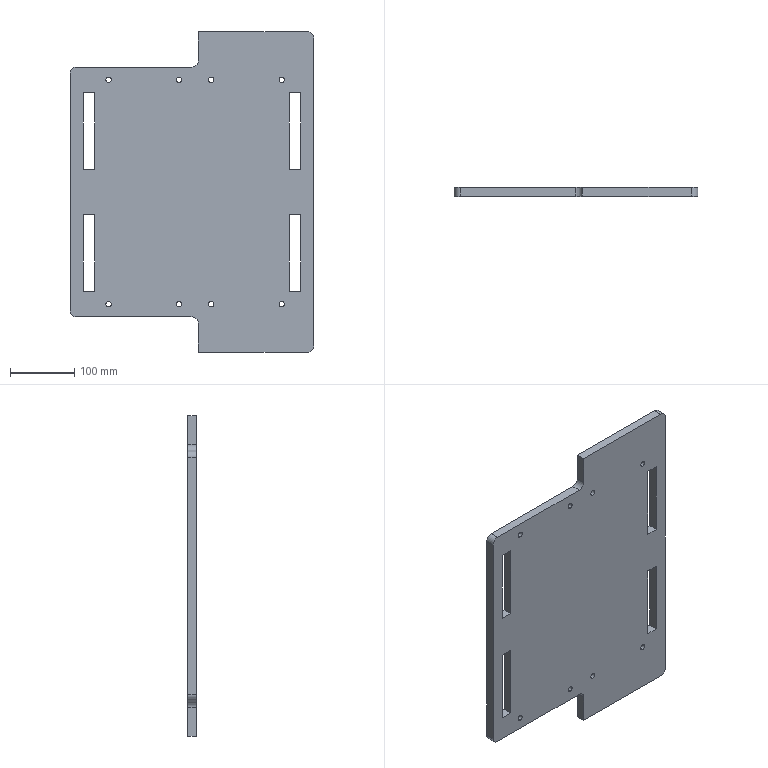Part | SolidWorks | features Fillet 2, ICE 2, Extrusion 1, HoleWzd 1, LPattern 1 | 1 solid | 48 faces | box 380 x 14 x 500 mm | volume 2220724 mm3 | plane 26 | cylinder 22 | commonest cylinder face diameters 8.5 x16 20 x6
STEP:
#1=CARTESIAN_POINT('',(-20.,0.,170.75));
#2=VERTEX_POINT('',#1);
#3=CARTESIAN_POINT('',(-20.,0.,179.25));
#4=VERTEX_POINT('',#3);
#5=CARTESIAN_POINT('',(-20.,0.,175.));
#6=DIRECTION('',(0.,1.,0.));
#7=DIRECTION('',(0.,0.,1.));
#8=AXIS2_PLACEMENT_3D('',#5,#6,#7);
#9=CIRCLE('',#8,4.25);
#10=EDGE_CURVE('',#2,#4,#9,.T.);
#11=ORIENTED_EDGE('',*,*,#10,.F.);
#12=CARTESIAN_POINT('',(-20.,14.,170.75));
#13=VERTEX_POINT('',#12);
#14=CARTESIAN_POINT('',(-20.,14.,170.75));
#15=DIRECTION('',(0.,1.,0.));
#16=VECTOR('',#15,1000.);
#17=LINE('',#14,#16);
#18=EDGE_CURVE('',#2,#13,#17,.T.);
#19=ORIENTED_EDGE('',*,*,#18,.T.);
#20=CARTESIAN_POINT('',(-20.,14.,179.25));
#21=VERTEX_POINT('',#20);
#22=CARTESIAN_POINT('',(-20.,14.,175.));
#23=DIRECTION('',(0.,1.,0.));
#24=DIRECTION('',(0.,0.,1.));
#25=AXIS2_PLACEMENT_3D('',#22,#23,#24);
#26=CIRCLE('',#25,4.25);
#27=EDGE_CURVE('',#13,#21,#26,.T.);
#28=ORIENTED_EDGE('',*,*,#27,.T.);
#29=CARTESIAN_POINT('',(-20.,14.,179.25));
#30=DIRECTION('',(0.,1.,0.));
#31=VECTOR('',#30,1000.);
#32=LINE('',#29,#31);
#33=EDGE_CURVE('',#4,#21,#32,.T.);
#34=ORIENTED_EDGE('',*,*,#33,.F.);
#35=EDGE_LOOP('',(#11,#19,#28,#34));
#36=FACE_OUTER_BOUND('',#35,.T.);
#37=CARTESIAN_POINT('',(-20.,14.,175.));
#38=DIRECTION('',(0.,1.,0.));
#39=DIRECTION('',(0.,0.,1.));
#40=AXIS2_PLACEMENT_3D('',#37,#38,#39);
#41=CYLINDRICAL_SURFACE('',#40,4.25);
#42=ADVANCED_FACE('',(#36),#41,.F.);
#43=CARTESIAN_POINT('',(-20.,0.,-179.25));
#44=VERTEX_POINT('',#43);
#45=CARTESIAN_POINT('',(-20.,0.,-170.75));
#46=VERTEX_POINT('',#45);
#47=CARTESIAN_POINT('',(-20.,0.,-175.));
#48=DIRECTION('',(0.,1.,0.));
#49=DIRECTION('',(0.,0.,1.));
#50=AXIS2_PLACEMENT_3D('',#47,#48,#49);
#51=CIRCLE('',#50,4.25);
#52=EDGE_CURVE('',#44,#46,#51,.T.);
#53=ORIENTED_EDGE('',*,*,#52,.F.);
#54=CARTESIAN_POINT('',(-20.,14.,-179.25));
#55=VERTEX_POINT('',#54);
#56=CARTESIAN_POINT('',(-20.,14.,-179.25));
#57=DIRECTION('',(0.,1.,0.));
#58=VECTOR('',#57,1000.);
#59=LINE('',#56,#58);
#60=EDGE_CURVE('',#44,#55,#59,.T.);
#61=ORIENTED_EDGE('',*,*,#60,.T.);
#62=CARTESIAN_POINT('',(-20.,14.,-170.75));
#63=VERTEX_POINT('',#62);
#64=CARTESIAN_POINT('',(-20.,14.,-175.));
#65=DIRECTION('',(0.,1.,0.));
#66=DIRECTION('',(0.,0.,1.));
#67=AXIS2_PLACEMENT_3D('',#64,#65,#66);
#68=CIRCLE('',#67,4.25);
#69=EDGE_CURVE('',#55,#63,#68,.T.);
#70=ORIENTED_EDGE('',*,*,#69,.T.);
#71=CARTESIAN_POINT('',(-20.,14.,-170.75));
#72=DIRECTION('',(0.,1.,0.));
#73=VECTOR('',#72,1000.);
#74=LINE('',#71,#73);
#75=EDGE_CURVE('',#46,#63,#74,.T.);
#76=ORIENTED_EDGE('',*,*,#75,.F.);
#77=EDGE_LOOP('',(#53,#61,#70,#76));
#78=FACE_OUTER_BOUND('',#77,.T.);
#79=CARTESIAN_POINT('',(-20.,14.,-175.));
#80=DIRECTION('',(0.,1.,0.));
#81=DIRECTION('',(0.,0.,1.));
#82=AXIS2_PLACEMENT_3D('',#79,#80,#81);
#83=CYLINDRICAL_SURFACE('',#82,4.25);
#84=ADVANCED_FACE('',(#78),#83,.F.);
#85=CARTESIAN_POINT('',(-130.,0.,-179.25));
#86=VERTEX_POINT('',#85);
#87=CARTESIAN_POINT('',(-130.,0.,-170.75));
#88=VERTEX_POINT('',#87);
#89=CARTESIAN_POINT('',(-130.,0.,-175.));
#90=DIRECTION('',(0.,1.,0.));
#91=DIRECTION('',(0.,0.,1.));
#92=AXIS2_PLACEMENT_3D('',#89,#90,#91);
#93=CIRCLE('',#92,4.25);
#94=EDGE_CURVE('',#86,#88,#93,.T.);
#95=ORIENTED_EDGE('',*,*,#94,.F.);
#96=CARTESIAN_POINT('',(-130.,14.,-179.25));
#97=VERTEX_POINT('',#96);
#98=CARTESIAN_POINT('',(-130.,14.,-179.25));
#99=DIRECTION('',(0.,1.,0.));
#100=VECTOR('',#99,1000.);
#101=LINE('',#98,#100);
#102=EDGE_CURVE('',#86,#97,#101,.T.);
#103=ORIENTED_EDGE('',*,*,#102,.T.);
#104=CARTESIAN_POINT('',(-130.,14.,-170.75));
#105=VERTEX_POINT('',#104);
#106=CARTESIAN_POINT('',(-130.,14.,-175.));
#107=DIRECTION('',(0.,1.,0.));
#108=DIRECTION('',(0.,0.,1.));
#109=AXIS2_PLACEMENT_3D('',#106,#107,#108);
#110=CIRCLE('',#109,4.25);
#111=EDGE_CURVE('',#97,#105,#110,.T.);
#112=ORIENTED_EDGE('',*,*,#111,.T.);
#113=CARTESIAN_POINT('',(-130.,14.,-170.75));
#114=DIRECTION('',(0.,1.,0.));
#115=VECTOR('',#114,1000.);
#116=LINE('',#113,#115);
#117=EDGE_CURVE('',#88,#105,#116,.T.);
#118=ORIENTED_EDGE('',*,*,#117,.F.);
#119=EDGE_LOOP('',(#95,#103,#112,#118));
#120=FACE_OUTER_BOUND('',#119,.T.);
#121=CARTESIAN_POINT('',(-130.,14.,-175.));
#122=DIRECTION('',(0.,1.,0.));
#123=DIRECTION('',(0.,0.,1.));
#124=AXIS2_PLACEMENT_3D('',#121,#122,#123);
#125=CYLINDRICAL_SURFACE('',#124,4.25);
#126=ADVANCED_FACE('',(#120),#125,.F.);
#127=CARTESIAN_POINT('',(-130.,0.,170.75));
#128=VERTEX_POINT('',#127);
#129=CARTESIAN_POINT('',(-130.,0.,179.25));
#130=VERTEX_POINT('',#129);
#131=CARTESIAN_POINT('',(-130.,0.,175.));
#132=DIRECTION('',(0.,1.,0.));
#133=DIRECTION('',(0.,0.,1.));
#134=AXIS2_PLACEMENT_3D('',#131,#132,#133);
#135=CIRCLE('',#134,4.25);
#136=EDGE_CURVE('',#128,#130,#135,.T.);
#137=ORIENTED_EDGE('',*,*,#136,.F.);
#138=CARTESIAN_POINT('',(-130.,14.,170.75));
#139=VERTEX_POINT('',#138);
#140=CARTESIAN_POINT('',(-130.,14.,170.75));
#141=DIRECTION('',(0.,1.,0.));
#142=VECTOR('',#141,1000.);
#143=LINE('',#140,#142);
#144=EDGE_CURVE('',#128,#139,#143,.T.);
#145=ORIENTED_EDGE('',*,*,#144,.T.);
#146=CARTESIAN_POINT('',(-130.,14.,179.25));
#147=VERTEX_POINT('',#146);
#148=CARTESIAN_POINT('',(-130.,14.,175.));
#149=DIRECTION('',(0.,1.,0.));
#150=DIRECTION('',(0.,0.,1.));
#151=AXIS2_PLACEMENT_3D('',#148,#149,#150);
#152=CIRCLE('',#151,4.25);
#153=EDGE_CURVE('',#139,#147,#152,.T.);
#154=ORIENTED_EDGE('',*,*,#153,.T.);
#155=CARTESIAN_POINT('',(-130.,14.,179.25));
#156=DIRECTION('',(0.,1.,0.));
#157=VECTOR('',#156,1000.);
#158=LINE('',#155,#157);
#159=EDGE_CURVE('',#130,#147,#158,.T.);
#160=ORIENTED_EDGE('',*,*,#159,.F.);
#161=EDGE_LOOP('',(#137,#145,#154,#160));
#162=FACE_OUTER_BOUND('',#161,.T.);
#163=CARTESIAN_POINT('',(-130.,14.,175.));
#164=DIRECTION('',(0.,1.,0.));
#165=DIRECTION('',(0.,0.,1.));
#166=AXIS2_PLACEMENT_3D('',#163,#164,#165);
#167=CYLINDRICAL_SURFACE('',#166,4.25);
#168=ADVANCED_FACE('',(#162),#167,.F.);
#169=CARTESIAN_POINT('',(30.,0.,170.75));
#170=VERTEX_POINT('',#169);
#171=CARTESIAN_POINT('',(30.,0.,179.25));
#172=VERTEX_POINT('',#171);
#173=CARTESIAN_POINT('',(30.,0.,175.));
#174=DIRECTION('',(0.,1.,0.));
#175=DIRECTION('',(0.,0.,1.));
#176=AXIS2_PLACEMENT_3D('',#173,#174,#175);
#177=CIRCLE('',#176,4.25);
#178=EDGE_CURVE('',#170,#172,#177,.T.);
#179=ORIENTED_EDGE('',*,*,#178,.F.);
#180=CARTESIAN_POINT('',(30.,14.,170.75));
#181=VERTEX_POINT('',#180);
#182=CARTESIAN_POINT('',(30.,14.,170.75));
#183=DIRECTION('',(0.,1.,0.));
#184=VECTOR('',#183,1000.);
#185=LINE('',#182,#184);
#186=EDGE_CURVE('',#170,#181,#185,.T.);
#187=ORIENTED_EDGE('',*,*,#186,.T.);
#188=CARTESIAN_POINT('',(30.,14.,179.25));
#189=VERTEX_POINT('',#188);
#190=CARTESIAN_POINT('',(30.,14.,175.));
#191=DIRECTION('',(0.,1.,0.));
#192=DIRECTION('',(0.,0.,1.));
#193=AXIS2_PLACEMENT_3D('',#190,#191,#192);
#194=CIRCLE('',#193,4.25);
#195=EDGE_CURVE('',#181,#189,#194,.T.);
#196=ORIENTED_EDGE('',*,*,#195,.T.);
#197=CARTESIAN_POINT('',(30.,14.,179.25));
#198=DIRECTION('',(0.,1.,0.));
#199=VECTOR('',#198,1000.);
#200=LINE('',#197,#199);
#201=EDGE_CURVE('',#172,#189,#200,.T.);
#202=ORIENTED_EDGE('',*,*,#201,.F.);
#203=EDGE_LOOP('',(#179,#187,#196,#202));
#204=FACE_OUTER_BOUND('',#203,.T.);
#205=CARTESIAN_POINT('',(30.,14.,175.));
#206=DIRECTION('',(0.,1.,0.));
#207=DIRECTION('',(0.,0.,1.));
#208=AXIS2_PLACEMENT_3D('',#205,#206,#207);
#209=CYLINDRICAL_SURFACE('',#208,4.25);
#210=ADVANCED_FACE('',(#204),#209,.F.);
#211=CARTESIAN_POINT('',(140.,0.,170.75));
#212=VERTEX_POINT('',#211);
#213=CARTESIAN_POINT('',(140.,0.,179.25));
#214=VERTEX_POINT('',#213);
#215=CARTESIAN_POINT('',(140.,0.,175.));
#216=DIRECTION('',(0.,1.,0.));
#217=DIRECTION('',(0.,0.,1.));
#218=AXIS2_PLACEMENT_3D('',#215,#216,#217);
#219=CIRCLE('',#218,4.25);
#220=EDGE_CURVE('',#212,#214,#219,.T.);
#221=ORIENTED_EDGE('',*,*,#220,.F.);
#222=CARTESIAN_POINT('',(140.,14.,170.75));
#223=VERTEX_POINT('',#222);
#224=CARTESIAN_POINT('',(140.,14.,170.75));
#225=DIRECTION('',(0.,1.,0.));
#226=VECTOR('',#225,1000.);
#227=LINE('',#224,#226);
#228=EDGE_CURVE('',#212,#223,#227,.T.);
#229=ORIENTED_EDGE('',*,*,#228,.T.);
#230=CARTESIAN_POINT('',(140.,14.,179.25));
#231=VERTEX_POINT('',#230);
#232=CARTESIAN_POINT('',(140.,14.,175.));
#233=DIRECTION('',(0.,1.,0.));
#234=DIRECTION('',(0.,0.,1.));
#235=AXIS2_PLACEMENT_3D('',#232,#233,#234);
#236=CIRCLE('',#235,4.25);
#237=EDGE_CURVE('',#223,#231,#236,.T.);
#238=ORIENTED_EDGE('',*,*,#237,.T.);
#239=CARTESIAN_POINT('',(140.,14.,179.25));
#240=DIRECTION('',(0.,1.,0.));
#241=VECTOR('',#240,1000.);
#242=LINE('',#239,#241);
#243=EDGE_CURVE('',#214,#231,#242,.T.);
#244=ORIENTED_EDGE('',*,*,#243,.F.);
#245=EDGE_LOOP('',(#221,#229,#238,#244));
#246=FACE_OUTER_BOUND('',#245,.T.);
#247=CARTESIAN_POINT('',(140.,14.,175.));
#248=DIRECTION('',(0.,1.,0.));
#249=DIRECTION('',(0.,0.,1.));
#250=AXIS2_PLACEMENT_3D('',#247,#248,#249);
#251=CYLINDRICAL_SURFACE('',#250,4.25);
#252=ADVANCED_FACE('',(#246),#251,.F.);
#253=CARTESIAN_POINT('',(140.,0.,-179.25));
#254=VERTEX_POINT('',#253);
#255=CARTESIAN_POINT('',(140.,0.,-170.75));
#256=VERTEX_POINT('',#255);
#257=CARTESIAN_POINT('',(140.,0.,-175.));
#258=DIRECTION('',(0.,1.,0.));
#259=DIRECTION('',(0.,0.,1.));
#260=AXIS2_PLACEMENT_3D('',#257,#258,#259);
#261=CIRCLE('',#260,4.25);
#262=EDGE_CURVE('',#254,#256,#261,.T.);
#263=ORIENTED_EDGE('',*,*,#262,.F.);
#264=CARTESIAN_POINT('',(140.,14.,-179.25));
#265=VERTEX_POINT('',#264);
#266=CARTESIAN_POINT('',(140.,14.,-179.25));
#267=DIRECTION('',(0.,1.,0.));
#268=VECTOR('',#267,1000.);
#269=LINE('',#266,#268);
#270=EDGE_CURVE('',#254,#265,#269,.T.);
#271=ORIENTED_EDGE('',*,*,#270,.T.);
#272=CARTESIAN_POINT('',(140.,14.,-170.75));
#273=VERTEX_POINT('',#272);
#274=CARTESIAN_POINT('',(140.,14.,-175.));
#275=DIRECTION('',(0.,1.,0.));
#276=DIRECTION('',(0.,0.,1.));
#277=AXIS2_PLACEMENT_3D('',#274,#275,#276);
#278=CIRCLE('',#277,4.25);
#279=EDGE_CURVE('',#265,#273,#278,.T.);
#280=ORIENTED_EDGE('',*,*,#279,.T.);
#281=CARTESIAN_POINT('',(140.,14.,-170.75));
#282=DIRECTION('',(0.,1.,0.));
#283=VECTOR('',#282,1000.);
#284=LINE('',#281,#283);
#285=EDGE_CURVE('',#256,#273,#284,.T.);
#286=ORIENTED_EDGE('',*,*,#285,.F.);
#287=EDGE_LOOP('',(#263,#271,#280,#286));
#288=FACE_OUTER_BOUND('',#287,.T.);
#289=CARTESIAN_POINT('',(140.,14.,-175.));
#290=DIRECTION('',(0.,1.,0.));
#291=DIRECTION('',(0.,0.,1.));
#292=AXIS2_PLACEMENT_3D('',#289,#290,#291);
#293=CYLINDRICAL_SURFACE('',#292,4.25);
#294=ADVANCED_FACE('',(#288),#293,.F.);
#295=CARTESIAN_POINT('',(30.,0.,-179.25));
#296=VERTEX_POINT('',#295);
#297=CARTESIAN_POINT('',(30.,0.,-170.75));
#298=VERTEX_POINT('',#297);
#299=CARTESIAN_POINT('',(30.,0.,-175.));
#300=DIRECTION('',(0.,1.,0.));
#301=DIRECTION('',(0.,0.,1.));
#302=AXIS2_PLACEMENT_3D('',#299,#300,#301);
#303=CIRCLE('',#302,4.25);
#304=EDGE_CURVE('',#296,#298,#303,.T.);
#305=ORIENTED_EDGE('',*,*,#304,.F.);
#306=CARTESIAN_POINT('',(30.,14.,-179.25));
#307=VERTEX_POINT('',#306);
#308=CARTESIAN_POINT('',(30.,14.,-179.25));
#309=DIRECTION('',(0.,1.,0.));
#310=VECTOR('',#309,1000.);
#311=LINE('',#308,#310);
#312=EDGE_CURVE('',#296,#307,#311,.T.);
#313=ORIENTED_EDGE('',*,*,#312,.T.);
#314=CARTESIAN_POINT('',(30.,14.,-170.75));
#315=VERTEX_POINT('',#314);
#316=CARTESIAN_POINT('',(30.,14.,-175.));
#317=DIRECTION('',(0.,1.,0.));
#318=DIRECTION('',(0.,0.,1.));
#319=AXIS2_PLACEMENT_3D('',#316,#317,#318);
#320=CIRCLE('',#319,4.25);
#321=EDGE_CURVE('',#307,#315,#320,.T.);
#322=ORIENTED_EDGE('',*,*,#321,.T.);
#323=CARTESIAN_POINT('',(30.,14.,-170.75));
#324=DIRECTION('',(0.,1.,0.));
#325=VECTOR('',#324,1000.);
#326=LINE('',#323,#325);
#327=EDGE_CURVE('',#298,#315,#326,.T.);
#328=ORIENTED_EDGE('',*,*,#327,.F.);
#329=EDGE_LOOP('',(#305,#313,#322,#328));
#330=FACE_OUTER_BOUND('',#329,.T.);
#331=CARTESIAN_POINT('',(30.,14.,-175.));
#332=DIRECTION('',(0.,1.,0.));
#333=DIRECTION('',(0.,0.,1.));
#334=AXIS2_PLACEMENT_3D('',#331,#332,#333);
#335=CYLINDRICAL_SURFACE('',#334,4.25);
#336=ADVANCED_FACE('',(#330),#335,.F.);
#337=CARTESIAN_POINT('',(190.,14.,240.));
#338=VERTEX_POINT('',#337);
#339=CARTESIAN_POINT('',(190.,14.,-240.));
#340=VERTEX_POINT('',#339);
#341=CARTESIAN_POINT('',(190.,14.,-250.));
#342=DIRECTION('',(0.,0.,-1.));
#343=VECTOR('',#342,1000.);
#344=LINE('',#341,#343);
#345=EDGE_CURVE('',#338,#340,#344,.T.);
#346=ORIENTED_EDGE('',*,*,#345,.F.);
#347=CARTESIAN_POINT('',(190.,0.,240.));
#348=VERTEX_POINT('',#347);
#349=CARTESIAN_POINT('',(190.,14.,240.));
#350=DIRECTION('',(0.,-1.,0.));
#351=VECTOR('',#350,1000.);
#352=LINE('',#349,#351);
#353=EDGE_CURVE('',#338,#348,#352,.T.);
#354=ORIENTED_EDGE('',*,*,#353,.T.);
#355=CARTESIAN_POINT('',(190.,0.,-240.));
#356=VERTEX_POINT('',#355);
#357=CARTESIAN_POINT('',(190.,0.,-250.));
#358=DIRECTION('',(0.,0.,-1.));
#359=VECTOR('',#358,1000.);
#360=LINE('',#357,#359);
#361=EDGE_CURVE('',#348,#356,#360,.T.);
#362=ORIENTED_EDGE('',*,*,#361,.T.);
#363=CARTESIAN_POINT('',(190.,14.,-240.));
#364=DIRECTION('',(0.,1.,0.));
#365=VECTOR('',#364,1000.);
#366=LINE('',#363,#365);
#367=EDGE_CURVE('',#356,#340,#366,.T.);
#368=ORIENTED_EDGE('',*,*,#367,.T.);
#369=EDGE_LOOP('',(#346,#354,#362,#368));
#370=FACE_OUTER_BOUND('',#369,.T.);
#371=CARTESIAN_POINT('',(190.,14.,-250.));
#372=DIRECTION('',(-1.,0.,0.));
#373=DIRECTION('',(0.,0.,1.));
#374=AXIS2_PLACEMENT_3D('',#371,#372,#373);
#375=PLANE('',#374);
#376=ADVANCED_FACE('',(#370),#375,.F.);
#377=CARTESIAN_POINT('',(180.,14.,-250.));
#378=VERTEX_POINT('',#377);
#379=CARTESIAN_POINT('',(10.,14.,-250.));
#380=VERTEX_POINT('',#379);
#381=CARTESIAN_POINT('',(-190.,14.,-250.));
#382=DIRECTION('',(-1.,0.,0.));
#383=VECTOR('',#382,1000.);
#384=LINE('',#381,#383);
#385=EDGE_CURVE('',#378,#380,#384,.T.);
#386=ORIENTED_EDGE('',*,*,#385,.F.);
#387=CARTESIAN_POINT('',(180.,0.,-250.));
#388=VERTEX_POINT('',#387);
#389=CARTESIAN_POINT('',(180.,14.,-250.));
#390=DIRECTION('',(0.,-1.,0.));
#391=VECTOR('',#390,1000.);
#392=LINE('',#389,#391);
#393=EDGE_CURVE('',#378,#388,#392,.T.);
#394=ORIENTED_EDGE('',*,*,#393,.T.);
#395=CARTESIAN_POINT('',(10.,0.,-250.));
#396=VERTEX_POINT('',#395);
#397=CARTESIAN_POINT('',(-190.,0.,-250.));
#398=DIRECTION('',(-1.,0.,0.));
#399=VECTOR('',#398,1000.);
#400=LINE('',#397,#399);
#401=EDGE_CURVE('',#388,#396,#400,.T.);
#402=ORIENTED_EDGE('',*,*,#401,.T.);
#403=CARTESIAN_POINT('',(10.,0.,-250.));
#404=DIRECTION('',(0.,1.,0.));
#405=VECTOR('',#404,1000.);
#406=LINE('',#403,#405);
#407=EDGE_CURVE('',#396,#380,#406,.T.);
#408=ORIENTED_EDGE('',*,*,#407,.T.);
#409=EDGE_LOOP('',(#386,#394,#402,#408));
#410=FACE_OUTER_BOUND('',#409,.T.);
#411=CARTESIAN_POINT('',(-190.,14.,-250.));
#412=DIRECTION('',(0.,0.,1.));
#413=DIRECTION('',(1.,0.,0.));
#414=AXIS2_PLACEMENT_3D('',#411,#412,#413);
#415=PLANE('',#414);
#416=ADVANCED_FACE('',(#410),#415,.F.);
#417=CARTESIAN_POINT('',(-190.,0.,-185.));
#418=VERTEX_POINT('',#417);
#419=CARTESIAN_POINT('',(-190.,0.,185.));
#420=VERTEX_POINT('',#419);
#421=CARTESIAN_POINT('',(-190.,0.,-250.));
#422=DIRECTION('',(0.,0.,1.));
#423=VECTOR('',#422,1000.);
#424=LINE('',#421,#423);
#425=EDGE_CURVE('',#418,#420,#424,.T.);
#426=ORIENTED_EDGE('',*,*,#425,.T.);
#427=CARTESIAN_POINT('',(-190.,14.,185.));
#428=VERTEX_POINT('',#427);
#429=CARTESIAN_POINT('',(-190.,14.,185.));
#430=DIRECTION('',(0.,1.,0.));
#431=VECTOR('',#430,1000.);
#432=LINE('',#429,#431);
#433=EDGE_CURVE('',#420,#428,#432,.T.);
#434=ORIENTED_EDGE('',*,*,#433,.T.);
#435=CARTESIAN_POINT('',(-190.,14.,-185.));
#436=VERTEX_POINT('',#435);
#437=CARTESIAN_POINT('',(-190.,14.,-250.));
#438=DIRECTION('',(0.,0.,1.));
#439=VECTOR('',#438,1000.);
#440=LINE('',#437,#439);
#441=EDGE_CURVE('',#436,#428,#440,.T.);
#442=ORIENTED_EDGE('',*,*,#441,.F.);
#443=CARTESIAN_POINT('',(-190.,14.,-185.));
#444=DIRECTION('',(0.,-1.,0.));
#445=VECTOR('',#444,1000.);
#446=LINE('',#443,#445);
#447=EDGE_CURVE('',#436,#418,#446,.T.);
#448=ORIENTED_EDGE('',*,*,#447,.T.);
#449=EDGE_LOOP('',(#426,#434,#442,#448));
#450=FACE_OUTER_BOUND('',#449,.T.);
#451=CARTESIAN_POINT('',(-190.,14.,-250.));
#452=DIRECTION('',(1.,0.,0.));
#453=DIRECTION('',(0.,0.,-1.));
#454=AXIS2_PLACEMENT_3D('',#451,#452,#453);
#455=PLANE('',#454);
#456=ADVANCED_FACE('',(#450),#455,.F.);
#457=CARTESIAN_POINT('',(10.,0.,250.));
#458=VERTEX_POINT('',#457);
#459=CARTESIAN_POINT('',(180.,0.,250.));
#460=VERTEX_POINT('',#459);
#461=CARTESIAN_POINT('',(-190.,0.,250.));
#462=DIRECTION('',(1.,0.,0.));
#463=VECTOR('',#462,1000.);
#464=LINE('',#461,#463);
#465=EDGE_CURVE('',#458,#460,#464,.T.);
#466=ORIENTED_EDGE('',*,*,#465,.T.);
#467=CARTESIAN_POINT('',(180.,14.,250.));
#468=VERTEX_POINT('',#467);
#469=CARTESIAN_POINT('',(180.,14.,250.));
#470=DIRECTION('',(0.,1.,0.));
#471=VECTOR('',#470,1000.);
#472=LINE('',#469,#471);
#473=EDGE_CURVE('',#460,#468,#472,.T.);
#474=ORIENTED_EDGE('',*,*,#473,.T.);
#475=CARTESIAN_POINT('',(10.,14.,250.));
#476=VERTEX_POINT('',#475);
#477=CARTESIAN_POINT('',(-190.,14.,250.));
#478=DIRECTION('',(1.,0.,0.));
#479=VECTOR('',#478,1000.);
#480=LINE('',#477,#479);
#481=EDGE_CURVE('',#476,#468,#480,.T.);
#482=ORIENTED_EDGE('',*,*,#481,.F.);
#483=CARTESIAN_POINT('',(10.,0.,250.));
#484=DIRECTION('',(0.,1.,0.));
#485=VECTOR('',#484,1000.);
#486=LINE('',#483,#485);
#487=EDGE_CURVE('',#458,#476,#486,.T.);
#488=ORIENTED_EDGE('',*,*,#487,.F.);
#489=EDGE_LOOP('',(#466,#474,#482,#488));
#490=FACE_OUTER_BOUND('',#489,.T.);
#491=CARTESIAN_POINT('',(-190.,14.,250.));
#492=DIRECTION('',(0.,0.,-1.));
#493=DIRECTION('',(-1.,0.,0.));
#494=AXIS2_PLACEMENT_3D('',#491,#492,#493);
#495=PLANE('',#494);
#496=ADVANCED_FACE('',(#490),#495,.F.);
#497=CARTESIAN_POINT('',(-20.,14.,175.));
#498=DIRECTION('',(0.,1.,0.));
#499=DIRECTION('',(0.,0.,1.));
#500=AXIS2_PLACEMENT_3D('',#497,#498,#499);
#501=CIRCLE('',#500,4.25);
#502=EDGE_CURVE('',#21,#13,#501,.T.);
#503=ORIENTED_EDGE('',*,*,#502,.F.);
#504=ORIENTED_EDGE('',*,*,#27,.F.);
#505=EDGE_LOOP('',(#503,#504));
#506=FACE_BOUND('',#505,.T.);
#507=CARTESIAN_POINT('',(-20.,14.,-175.));
#508=DIRECTION('',(0.,1.,0.));
#509=DIRECTION('',(0.,0.,1.));
#510=AXIS2_PLACEMENT_3D('',#507,#508,#509);
#511=CIRCLE('',#510,4.25);
#512=EDGE_CURVE('',#63,#55,#511,.T.);
#513=ORIENTED_EDGE('',*,*,#512,.F.);
#514=ORIENTED_EDGE('',*,*,#69,.F.);
#515=EDGE_LOOP('',(#513,#514));
#516=FACE_BOUND('',#515,.T.);
#517=CARTESIAN_POINT('',(-130.,14.,-175.));
#518=DIRECTION('',(0.,1.,0.));
#519=DIRECTION('',(0.,0.,1.));
#520=AXIS2_PLACEMENT_3D('',#517,#518,#519);
#521=CIRCLE('',#520,4.25);
#522=EDGE_CURVE('',#105,#97,#521,.T.);
#523=ORIENTED_EDGE('',*,*,#522,.F.);
#524=ORIENTED_EDGE('',*,*,#111,.F.);
#525=EDGE_LOOP('',(#523,#524));
#526=FACE_BOUND('',#525,.T.);
#527=CARTESIAN_POINT('',(-130.,14.,175.));
#528=DIRECTION('',(0.,1.,0.));
#529=DIRECTION('',(0.,0.,1.));
#530=AXIS2_PLACEMENT_3D('',#527,#528,#529);
#531=CIRCLE('',#530,4.25);
#532=EDGE_CURVE('',#147,#139,#531,.T.);
#533=ORIENTED_EDGE('',*,*,#532,.F.);
#534=ORIENTED_EDGE('',*,*,#153,.F.);
#535=EDGE_LOOP('',(#533,#534));
#536=FACE_BOUND('',#535,.T.);
#537=CARTESIAN_POINT('',(30.,14.,175.));
#538=DIRECTION('',(0.,1.,0.));
#539=DIRECTION('',(0.,0.,1.));
#540=AXIS2_PLACEMENT_3D('',#537,#538,#539);
#541=CIRCLE('',#540,4.25);
#542=EDGE_CURVE('',#189,#181,#541,.T.);
#543=ORIENTED_EDGE('',*,*,#542,.F.);
#544=ORIENTED_EDGE('',*,*,#195,.F.);
#545=EDGE_LOOP('',(#543,#544));
#546=FACE_BOUND('',#545,.T.);
#547=CARTESIAN_POINT('',(140.,14.,175.));
#548=DIRECTION('',(0.,1.,0.));
#549=DIRECTION('',(0.,0.,1.));
#550=AXIS2_PLACEMENT_3D('',#547,#548,#549);
#551=CIRCLE('',#550,4.25);
#552=EDGE_CURVE('',#231,#223,#551,.T.);
#553=ORIENTED_EDGE('',*,*,#552,.F.);
#554=ORIENTED_EDGE('',*,*,#237,.F.);
#555=EDGE_LOOP('',(#553,#554));
#556=FACE_BOUND('',#555,.T.);
#557=CARTESIAN_POINT('',(140.,14.,-175.));
#558=DIRECTION('',(0.,1.,0.));
#559=DIRECTION('',(0.,0.,1.));
#560=AXIS2_PLACEMENT_3D('',#557,#558,#559);
#561=CIRCLE('',#560,4.25);
#562=EDGE_CURVE('',#273,#265,#561,.T.);
#563=ORIENTED_EDGE('',*,*,#562,.F.);
#564=ORIENTED_EDGE('',*,*,#279,.F.);
#565=EDGE_LOOP('',(#563,#564));
#566=FACE_BOUND('',#565,.T.);
#567=CARTESIAN_POINT('',(30.,14.,-175.));
#568=DIRECTION('',(0.,1.,0.));
#569=DIRECTION('',(0.,0.,1.));
#570=AXIS2_PLACEMENT_3D('',#567,#568,#569);
#571=CIRCLE('',#570,4.25);
#572=EDGE_CURVE('',#315,#307,#571,.T.);
#573=ORIENTED_EDGE('',*,*,#572,.F.);
#574=ORIENTED_EDGE('',*,*,#321,.F.);
#575=EDGE_LOOP('',(#573,#574));
#576=FACE_BOUND('',#575,.T.);
#577=CARTESIAN_POINT('',(-151.5,14.,-155.));
#578=VERTEX_POINT('',#577);
#579=CARTESIAN_POINT('',(-170.,14.,-155.));
#580=VERTEX_POINT('',#579);
#581=CARTESIAN_POINT('',(-151.5,14.,-155.));
#582=DIRECTION('',(-1.,0.,0.));
#583=VECTOR('',#582,1000.);
#584=LINE('',#581,#583);
#585=EDGE_CURVE('',#578,#580,#584,.T.);
#586=ORIENTED_EDGE('',*,*,#585,.F.);
#587=CARTESIAN_POINT('',(-151.5,14.,-35.));
#588=VERTEX_POINT('',#587);
#589=CARTESIAN_POINT('',(-151.5,14.,-155.));
#590=DIRECTION('',(0.,0.,-1.));
#591=VECTOR('',#590,1000.);
#592=LINE('',#589,#591);
#593=EDGE_CURVE('',#588,#578,#592,.T.);
#594=ORIENTED_EDGE('',*,*,#593,.F.);
#595=CARTESIAN_POINT('',(-170.,14.,-35.));
#596=VERTEX_POINT('',#595);
#597=CARTESIAN_POINT('',(-151.5,14.,-35.));
#598=DIRECTION('',(1.,0.,0.));
#599=VECTOR('',#598,1000.);
#600=LINE('',#597,#599);
#601=EDGE_CURVE('',#596,#588,#600,.T.);
#602=ORIENTED_EDGE('',*,*,#601,.F.);
#603=CARTESIAN_POINT('',(-170.,14.,-155.));
#604=DIRECTION('',(0.,0.,1.));
#605=VECTOR('',#604,1000.);
#606=LINE('',#603,#605);
#607=EDGE_CURVE('',#580,#596,#606,.T.);
#608=ORIENTED_EDGE('',*,*,#607,.F.);
#609=EDGE_LOOP('',(#586,#594,#602,#608));
#610=FACE_BOUND('',#609,.T.);
#611=CARTESIAN_POINT('',(-151.5,14.,155.));
#612=VERTEX_POINT('',#611);
#613=CARTESIAN_POINT('',(-151.5,14.,35.));
#614=VERTEX_POINT('',#613);
#615=CARTESIAN_POINT('',(-151.5,14.,155.));
#616=DIRECTION('',(0.,0.,-1.));
#617=VECTOR('',#616,1000.);
#618=LINE('',#615,#617);
#619=EDGE_CURVE('',#612,#614,#618,.T.);
#620=ORIENTED_EDGE('',*,*,#619,.F.);
#621=CARTESIAN_POINT('',(-170.,14.,155.));
#622=VERTEX_POINT('',#621);
#623=CARTESIAN_POINT('',(-151.5,14.,155.));
#624=DIRECTION('',(1.,0.,0.));
#625=VECTOR('',#624,1000.);
#626=LINE('',#623,#625);
#627=EDGE_CURVE('',#622,#612,#626,.T.);
#628=ORIENTED_EDGE('',*,*,#627,.F.);
#629=CARTESIAN_POINT('',(-170.,14.,35.));
#630=VERTEX_POINT('',#629);
#631=CARTESIAN_POINT('',(-170.,14.,155.));
#632=DIRECTION('',(0.,0.,1.));
#633=VECTOR('',#632,1000.);
#634=LINE('',#631,#633);
#635=EDGE_CURVE('',#630,#622,#634,.T.);
#636=ORIENTED_EDGE('',*,*,#635,.F.);
#637=CARTESIAN_POINT('',(-151.5,14.,35.));
#638=DIRECTION('',(-1.,0.,0.));
#639=VECTOR('',#638,1000.);
#640=LINE('',#637,#639);
#641=EDGE_CURVE('',#614,#630,#640,.T.);
#642=ORIENTED_EDGE('',*,*,#641,.F.);
#643=EDGE_LOOP('',(#620,#628,#636,#642));
#644=FACE_BOUND('',#643,.T.);
#645=CARTESIAN_POINT('',(151.5,14.,155.));
#646=VERTEX_POINT('',#645);
#647=CARTESIAN_POINT('',(170.,14.,155.));
#648=VERTEX_POINT('',#647);
#649=CARTESIAN_POINT('',(151.5,14.,155.));
#650=DIRECTION('',(1.,0.,0.));
#651=VECTOR('',#650,1000.);
#652=LINE('',#649,#651);
#653=EDGE_CURVE('',#646,#648,#652,.T.);
#654=ORIENTED_EDGE('',*,*,#653,.F.);
#655=CARTESIAN_POINT('',(151.5,14.,35.));
#656=VERTEX_POINT('',#655);
#657=CARTESIAN_POINT('',(151.5,14.,155.));
#658=DIRECTION('',(0.,0.,1.));
#659=VECTOR('',#658,1000.);
#660=LINE('',#657,#659);
#661=EDGE_CURVE('',#656,#646,#660,.T.);
#662=ORIENTED_EDGE('',*,*,#661,.F.);
#663=CARTESIAN_POINT('',(170.,14.,35.));
#664=VERTEX_POINT('',#663);
#665=CARTESIAN_POINT('',(151.5,14.,35.));
#666=DIRECTION('',(-1.,0.,0.));
#667=VECTOR('',#666,1000.);
#668=LINE('',#665,#667);
#669=EDGE_CURVE('',#664,#656,#668,.T.);
#670=ORIENTED_EDGE('',*,*,#669,.F.);
#671=CARTESIAN_POINT('',(170.,14.,155.));
#672=DIRECTION('',(0.,0.,-1.));
#673=VECTOR('',#672,1000.);
#674=LINE('',#671,#673);
#675=EDGE_CURVE('',#648,#664,#674,.T.);
#676=ORIENTED_EDGE('',*,*,#675,.F.);
#677=EDGE_LOOP('',(#654,#662,#670,#676));
#678=FACE_BOUND('',#677,.T.);
#679=CARTESIAN_POINT('',(151.5,14.,-155.));
#680=VERTEX_POINT('',#679);
#681=CARTESIAN_POINT('',(151.5,14.,-35.));
#682=VERTEX_POINT('',#681);
#683=CARTESIAN_POINT('',(151.5,14.,-155.));
#684=DIRECTION('',(0.,0.,1.));
#685=VECTOR('',#684,1000.);
#686=LINE('',#683,#685);
#687=EDGE_CURVE('',#680,#682,#686,.T.);
#688=ORIENTED_EDGE('',*,*,#687,.F.);
#689=CARTESIAN_POINT('',(170.,14.,-155.));
#690=VERTEX_POINT('',#689);
#691=CARTESIAN_POINT('',(151.5,14.,-155.));
#692=DIRECTION('',(-1.,0.,0.));
#693=VECTOR('',#692,1000.);
#694=LINE('',#691,#693);
#695=EDGE_CURVE('',#690,#680,#694,.T.);
#696=ORIENTED_EDGE('',*,*,#695,.F.);
#697=CARTESIAN_POINT('',(170.,14.,-35.));
#698=VERTEX_POINT('',#697);
#699=CARTESIAN_POINT('',(170.,14.,-155.));
#700=DIRECTION('',(0.,0.,-1.));
#701=VECTOR('',#700,1000.);
#702=LINE('',#699,#701);
#703=EDGE_CURVE('',#698,#690,#702,.T.);
#704=ORIENTED_EDGE('',*,*,#703,.F.);
#705=CARTESIAN_POINT('',(151.5,14.,-35.));
#706=DIRECTION('',(1.,0.,0.));
#707=VECTOR('',#706,1000.);
#708=LINE('',#705,#707);
#709=EDGE_CURVE('',#682,#698,#708,.T.);
#710=ORIENTED_EDGE('',*,*,#709,.F.);
#711=EDGE_LOOP('',(#688,#696,#704,#710));
#712=FACE_BOUND('',#711,.T.);
#713=ORIENTED_EDGE('',*,*,#481,.T.);
#714=CARTESIAN_POINT('',(180.,14.,240.));
#715=DIRECTION('',(0.,1.,0.));
#716=DIRECTION('',(0.,0.,1.));
#717=AXIS2_PLACEMENT_3D('',#714,#715,#716);
#718=CIRCLE('',#717,10.);
#719=EDGE_CURVE('',#468,#338,#718,.T.);
#720=ORIENTED_EDGE('',*,*,#719,.T.);
#721=ORIENTED_EDGE('',*,*,#345,.T.);
#722=CARTESIAN_POINT('',(180.,14.,-240.));
#723=DIRECTION('',(0.,1.,0.));
#724=DIRECTION('',(0.,0.,1.));
#725=AXIS2_PLACEMENT_3D('',#722,#723,#724);
#726=CIRCLE('',#725,10.);
#727=EDGE_CURVE('',#340,#378,#726,.T.);
#728=ORIENTED_EDGE('',*,*,#727,.T.);
#729=ORIENTED_EDGE('',*,*,#385,.T.);
#730=CARTESIAN_POINT('',(10.,14.,-205.));
#731=VERTEX_POINT('',#730);
#732=CARTESIAN_POINT('',(10.,14.,-250.));
#733=DIRECTION('',(0.,0.,-1.));
#734=VECTOR('',#733,1000.);
#735=LINE('',#732,#734);
#736=EDGE_CURVE('',#731,#380,#735,.T.);
#737=ORIENTED_EDGE('',*,*,#736,.F.);
#738=CARTESIAN_POINT('',(0.,14.,-195.));
#739=VERTEX_POINT('',#738);
#740=CARTESIAN_POINT('',(0.,14.,-205.));
#741=DIRECTION('',(0.,-1.,0.));
#742=DIRECTION('',(0.,0.,1.));
#743=AXIS2_PLACEMENT_3D('',#740,#741,#742);
#744=CIRCLE('',#743,10.);
#745=EDGE_CURVE('',#731,#739,#744,.T.);
#746=ORIENTED_EDGE('',*,*,#745,.T.);
#747=CARTESIAN_POINT('',(-180.,14.,-195.));
#748=VERTEX_POINT('',#747);
#749=CARTESIAN_POINT('',(-190.,14.,-195.));
#750=DIRECTION('',(1.,0.,0.));
#751=VECTOR('',#750,1000.);
#752=LINE('',#749,#751);
#753=EDGE_CURVE('',#748,#739,#752,.T.);
#754=ORIENTED_EDGE('',*,*,#753,.F.);
#755=CARTESIAN_POINT('',(-180.,14.,-185.));
#756=DIRECTION('',(0.,1.,0.));
#757=DIRECTION('',(0.,0.,1.));
#758=AXIS2_PLACEMENT_3D('',#755,#756,#757);
#759=CIRCLE('',#758,10.);
#760=EDGE_CURVE('',#748,#436,#759,.T.);
#761=ORIENTED_EDGE('',*,*,#760,.T.);
#762=ORIENTED_EDGE('',*,*,#441,.T.);
#763=CARTESIAN_POINT('',(-180.,14.,195.));
#764=VERTEX_POINT('',#763);
#765=CARTESIAN_POINT('',(-180.,14.,185.));
#766=DIRECTION('',(0.,1.,0.));
#767=DIRECTION('',(0.,0.,1.));
#768=AXIS2_PLACEMENT_3D('',#765,#766,#767);
#769=CIRCLE('',#768,10.);
#770=EDGE_CURVE('',#428,#764,#769,.T.);
#771=ORIENTED_EDGE('',*,*,#770,.T.);
#772=CARTESIAN_POINT('',(0.,14.,195.));
#773=VERTEX_POINT('',#772);
#774=CARTESIAN_POINT('',(-190.,14.,195.));
#775=DIRECTION('',(-1.,0.,0.));
#776=VECTOR('',#775,1000.);
#777=LINE('',#774,#776);
#778=EDGE_CURVE('',#773,#764,#777,.T.);
#779=ORIENTED_EDGE('',*,*,#778,.F.);
#780=CARTESIAN_POINT('',(10.,14.,205.));
#781=VERTEX_POINT('',#780);
#782=CARTESIAN_POINT('',(0.,14.,205.));
#783=DIRECTION('',(0.,-1.,0.));
#784=DIRECTION('',(0.,0.,1.));
#785=AXIS2_PLACEMENT_3D('',#782,#783,#784);
#786=CIRCLE('',#785,10.);
#787=EDGE_CURVE('',#773,#781,#786,.T.);
#788=ORIENTED_EDGE('',*,*,#787,.T.);
#789=CARTESIAN_POINT('',(10.,14.,250.));
#790=DIRECTION('',(0.,0.,-1.));
#791=VECTOR('',#790,1000.);
#792=LINE('',#789,#791);
#793=EDGE_CURVE('',#476,#781,#792,.T.);
#794=ORIENTED_EDGE('',*,*,#793,.F.);
#795=EDGE_LOOP('',(#713,#720,#721,#728,#729,#737,#746,#754,#761,#762,#771,#779,#788,#794));
#796=FACE_OUTER_BOUND('',#795,.T.);
#797=CARTESIAN_POINT('',(0.,14.,0.));
#798=DIRECTION('',(0.,1.,0.));
#799=DIRECTION('',(0.,0.,1.));
#800=AXIS2_PLACEMENT_3D('',#797,#798,#799);
#801=PLANE('',#800);
#802=ADVANCED_FACE('',(#506,#516,#526,#536,#546,#556,#566,#576,#610,#644,#678,#712,#796),#801,.T.);
#803=CARTESIAN_POINT('',(-20.,0.,175.));
#804=DIRECTION('',(0.,1.,0.));
#805=DIRECTION('',(0.,0.,1.));
#806=AXIS2_PLACEMENT_3D('',#803,#804,#805);
#807=CIRCLE('',#806,4.25);
#808=EDGE_CURVE('',#4,#2,#807,.T.);
#809=ORIENTED_EDGE('',*,*,#808,.T.);
#810=ORIENTED_EDGE('',*,*,#10,.T.);
#811=EDGE_LOOP('',(#809,#810));
#812=FACE_BOUND('',#811,.T.);
#813=CARTESIAN_POINT('',(-20.,0.,-175.));
#814=DIRECTION('',(0.,1.,0.));
#815=DIRECTION('',(0.,0.,1.));
#816=AXIS2_PLACEMENT_3D('',#813,#814,#815);
#817=CIRCLE('',#816,4.25);
#818=EDGE_CURVE('',#46,#44,#817,.T.);
#819=ORIENTED_EDGE('',*,*,#818,.T.);
#820=ORIENTED_EDGE('',*,*,#52,.T.);
#821=EDGE_LOOP('',(#819,#820));
#822=FACE_BOUND('',#821,.T.);
#823=CARTESIAN_POINT('',(-130.,0.,-175.));
#824=DIRECTION('',(0.,1.,0.));
#825=DIRECTION('',(0.,0.,1.));
#826=AXIS2_PLACEMENT_3D('',#823,#824,#825);
#827=CIRCLE('',#826,4.25);
#828=EDGE_CURVE('',#88,#86,#827,.T.);
#829=ORIENTED_EDGE('',*,*,#828,.T.);
#830=ORIENTED_EDGE('',*,*,#94,.T.);
#831=EDGE_LOOP('',(#829,#830));
#832=FACE_BOUND('',#831,.T.);
#833=CARTESIAN_POINT('',(-130.,0.,175.));
#834=DIRECTION('',(0.,1.,0.));
#835=DIRECTION('',(0.,0.,1.));
#836=AXIS2_PLACEMENT_3D('',#833,#834,#835);
#837=CIRCLE('',#836,4.25);
#838=EDGE_CURVE('',#130,#128,#837,.T.);
#839=ORIENTED_EDGE('',*,*,#838,.T.);
#840=ORIENTED_EDGE('',*,*,#136,.T.);
#841=EDGE_LOOP('',(#839,#840));
#842=FACE_BOUND('',#841,.T.);
#843=CARTESIAN_POINT('',(30.,0.,175.));
#844=DIRECTION('',(0.,1.,0.));
#845=DIRECTION('',(0.,0.,1.));
#846=AXIS2_PLACEMENT_3D('',#843,#844,#845);
#847=CIRCLE('',#846,4.25);
#848=EDGE_CURVE('',#172,#170,#847,.T.);
#849=ORIENTED_EDGE('',*,*,#848,.T.);
#850=ORIENTED_EDGE('',*,*,#178,.T.);
#851=EDGE_LOOP('',(#849,#850));
#852=FACE_BOUND('',#851,.T.);
#853=CARTESIAN_POINT('',(140.,0.,175.));
#854=DIRECTION('',(0.,1.,0.));
#855=DIRECTION('',(0.,0.,1.));
#856=AXIS2_PLACEMENT_3D('',#853,#854,#855);
#857=CIRCLE('',#856,4.25);
#858=EDGE_CURVE('',#214,#212,#857,.T.);
#859=ORIENTED_EDGE('',*,*,#858,.T.);
#860=ORIENTED_EDGE('',*,*,#220,.T.);
#861=EDGE_LOOP('',(#859,#860));
#862=FACE_BOUND('',#861,.T.);
#863=CARTESIAN_POINT('',(140.,0.,-175.));
#864=DIRECTION('',(0.,1.,0.));
#865=DIRECTION('',(0.,0.,1.));
#866=AXIS2_PLACEMENT_3D('',#863,#864,#865);
#867=CIRCLE('',#866,4.25);
#868=EDGE_CURVE('',#256,#254,#867,.T.);
#869=ORIENTED_EDGE('',*,*,#868,.T.);
#870=ORIENTED_EDGE('',*,*,#262,.T.);
#871=EDGE_LOOP('',(#869,#870));
#872=FACE_BOUND('',#871,.T.);
#873=CARTESIAN_POINT('',(30.,0.,-175.));
#874=DIRECTION('',(0.,1.,0.));
#875=DIRECTION('',(0.,0.,1.));
#876=AXIS2_PLACEMENT_3D('',#873,#874,#875);
#877=CIRCLE('',#876,4.25);
#878=EDGE_CURVE('',#298,#296,#877,.T.);
#879=ORIENTED_EDGE('',*,*,#878,.T.);
#880=ORIENTED_EDGE('',*,*,#304,.T.);
#881=EDGE_LOOP('',(#879,#880));
#882=FACE_BOUND('',#881,.T.);
#883=CARTESIAN_POINT('',(-151.5,0.,-35.));
#884=VERTEX_POINT('',#883);
#885=CARTESIAN_POINT('',(-151.5,0.,-155.));
#886=VERTEX_POINT('',#885);
#887=CARTESIAN_POINT('',(-151.5,0.,0.));
#888=DIRECTION('',(0.,0.,-1.));
#889=VECTOR('',#888,1000.);
#890=LINE('',#887,#889);
#891=EDGE_CURVE('',#884,#886,#890,.T.);
#892=ORIENTED_EDGE('',*,*,#891,.T.);
#893=CARTESIAN_POINT('',(-170.,0.,-155.));
#894=VERTEX_POINT('',#893);
#895=CARTESIAN_POINT('',(0.,0.,-155.));
#896=DIRECTION('',(-1.,0.,0.));
#897=VECTOR('',#896,1000.);
#898=LINE('',#895,#897);
#899=EDGE_CURVE('',#886,#894,#898,.T.);
#900=ORIENTED_EDGE('',*,*,#899,.T.);
#901=CARTESIAN_POINT('',(-170.,0.,-35.));
#902=VERTEX_POINT('',#901);
#903=CARTESIAN_POINT('',(-170.,0.,0.));
#904=DIRECTION('',(0.,0.,1.));
#905=VECTOR('',#904,1000.);
#906=LINE('',#903,#905);
#907=EDGE_CURVE('',#894,#902,#906,.T.);
#908=ORIENTED_EDGE('',*,*,#907,.T.);
#909=CARTESIAN_POINT('',(0.,0.,-35.));
#910=DIRECTION('',(1.,0.,0.));
#911=VECTOR('',#910,1000.);
#912=LINE('',#909,#911);
#913=EDGE_CURVE('',#902,#884,#912,.T.);
#914=ORIENTED_EDGE('',*,*,#913,.T.);
#915=EDGE_LOOP('',(#892,#900,#908,#914));
#916=FACE_BOUND('',#915,.T.);
#917=CARTESIAN_POINT('',(-170.,0.,155.));
#918=VERTEX_POINT('',#917);
#919=CARTESIAN_POINT('',(-151.5,0.,155.));
#920=VERTEX_POINT('',#919);
#921=CARTESIAN_POINT('',(0.,0.,155.));
#922=DIRECTION('',(1.,0.,0.));
#923=VECTOR('',#922,1000.);
#924=LINE('',#921,#923);
#925=EDGE_CURVE('',#918,#920,#924,.T.);
#926=ORIENTED_EDGE('',*,*,#925,.T.);
#927=CARTESIAN_POINT('',(-151.5,0.,35.));
#928=VERTEX_POINT('',#927);
#929=CARTESIAN_POINT('',(-151.5,0.,0.));
#930=DIRECTION('',(0.,0.,-1.));
#931=VECTOR('',#930,1000.);
#932=LINE('',#929,#931);
#933=EDGE_CURVE('',#920,#928,#932,.T.);
#934=ORIENTED_EDGE('',*,*,#933,.T.);
#935=CARTESIAN_POINT('',(-170.,0.,35.));
#936=VERTEX_POINT('',#935);
#937=CARTESIAN_POINT('',(0.,0.,35.));
#938=DIRECTION('',(-1.,0.,0.));
#939=VECTOR('',#938,1000.);
#940=LINE('',#937,#939);
#941=EDGE_CURVE('',#928,#936,#940,.T.);
#942=ORIENTED_EDGE('',*,*,#941,.T.);
#943=CARTESIAN_POINT('',(-170.,0.,0.));
#944=DIRECTION('',(0.,0.,1.));
#945=VECTOR('',#944,1000.);
#946=LINE('',#943,#945);
#947=EDGE_CURVE('',#936,#918,#946,.T.);
#948=ORIENTED_EDGE('',*,*,#947,.T.);
#949=EDGE_LOOP('',(#926,#934,#942,#948));
#950=FACE_BOUND('',#949,.T.);
#951=CARTESIAN_POINT('',(151.5,0.,35.));
#952=VERTEX_POINT('',#951);
#953=CARTESIAN_POINT('',(151.5,0.,155.));
#954=VERTEX_POINT('',#953);
#955=CARTESIAN_POINT('',(151.5,0.,0.));
#956=DIRECTION('',(0.,0.,1.));
#957=VECTOR('',#956,1000.);
#958=LINE('',#955,#957);
#959=EDGE_CURVE('',#952,#954,#958,.T.);
#960=ORIENTED_EDGE('',*,*,#959,.T.);
#961=CARTESIAN_POINT('',(170.,0.,155.));
#962=VERTEX_POINT('',#961);
#963=CARTESIAN_POINT('',(0.,0.,155.));
#964=DIRECTION('',(1.,0.,0.));
#965=VECTOR('',#964,1000.);
#966=LINE('',#963,#965);
#967=EDGE_CURVE('',#954,#962,#966,.T.);
#968=ORIENTED_EDGE('',*,*,#967,.T.);
#969=CARTESIAN_POINT('',(170.,0.,35.));
#970=VERTEX_POINT('',#969);
#971=CARTESIAN_POINT('',(170.,0.,0.));
#972=DIRECTION('',(0.,0.,-1.));
#973=VECTOR('',#972,1000.);
#974=LINE('',#971,#973);
#975=EDGE_CURVE('',#962,#970,#974,.T.);
#976=ORIENTED_EDGE('',*,*,#975,.T.);
#977=CARTESIAN_POINT('',(0.,0.,35.));
#978=DIRECTION('',(-1.,0.,0.));
#979=VECTOR('',#978,1000.);
#980=LINE('',#977,#979);
#981=EDGE_CURVE('',#970,#952,#980,.T.);
#982=ORIENTED_EDGE('',*,*,#981,.T.);
#983=EDGE_LOOP('',(#960,#968,#976,#982));
#984=FACE_BOUND('',#983,.T.);
#985=CARTESIAN_POINT('',(170.,0.,-155.));
#986=VERTEX_POINT('',#985);
#987=CARTESIAN_POINT('',(151.5,0.,-155.));
#988=VERTEX_POINT('',#987);
#989=CARTESIAN_POINT('',(0.,0.,-155.));
#990=DIRECTION('',(-1.,0.,0.));
#991=VECTOR('',#990,1000.);
#992=LINE('',#989,#991);
#993=EDGE_CURVE('',#986,#988,#992,.T.);
#994=ORIENTED_EDGE('',*,*,#993,.T.);
#995=CARTESIAN_POINT('',(151.5,0.,-35.));
#996=VERTEX_POINT('',#995);
#997=CARTESIAN_POINT('',(151.5,0.,0.));
#998=DIRECTION('',(0.,0.,1.));
#999=VECTOR('',#998,1000.);
#1000=LINE('',#997,#999);
#1001=EDGE_CURVE('',#988,#996,#1000,.T.);
#1002=ORIENTED_EDGE('',*,*,#1001,.T.);
#1003=CARTESIAN_POINT('',(170.,0.,-35.));
#1004=VERTEX_POINT('',#1003);
#1005=CARTESIAN_POINT('',(0.,0.,-35.));
#1006=DIRECTION('',(1.,0.,0.));
#1007=VECTOR('',#1006,1000.);
#1008=LINE('',#1005,#1007);
#1009=EDGE_CURVE('',#996,#1004,#1008,.T.);
#1010=ORIENTED_EDGE('',*,*,#1009,.T.);
#1011=CARTESIAN_POINT('',(170.,0.,0.));
#1012=DIRECTION('',(0.,0.,-1.));
#1013=VECTOR('',#1012,1000.);
#1014=LINE('',#1011,#1013);
#1015=EDGE_CURVE('',#1004,#986,#1014,.T.);
#1016=ORIENTED_EDGE('',*,*,#1015,.T.);
#1017=EDGE_LOOP('',(#994,#1002,#1010,#1016));
#1018=FACE_BOUND('',#1017,.T.);
#1019=ORIENTED_EDGE('',*,*,#361,.F.);
#1020=CARTESIAN_POINT('',(180.,0.,240.));
#1021=DIRECTION('',(0.,-1.,0.));
#1022=DIRECTION('',(0.,0.,1.));
#1023=AXIS2_PLACEMENT_3D('',#1020,#1021,#1022);
#1024=CIRCLE('',#1023,10.);
#1025=EDGE_CURVE('',#348,#460,#1024,.T.);
#1026=ORIENTED_EDGE('',*,*,#1025,.T.);
#1027=ORIENTED_EDGE('',*,*,#465,.F.);
#1028=CARTESIAN_POINT('',(10.,0.,205.));
#1029=VERTEX_POINT('',#1028);
#1030=CARTESIAN_POINT('',(10.,0.,250.));
#1031=DIRECTION('',(0.,0.,-1.));
#1032=VECTOR('',#1031,1000.);
#1033=LINE('',#1030,#1032);
#1034=EDGE_CURVE('',#458,#1029,#1033,.T.);
#1035=ORIENTED_EDGE('',*,*,#1034,.T.);
#1036=CARTESIAN_POINT('',(0.,0.,195.));
#1037=VERTEX_POINT('',#1036);
#1038=CARTESIAN_POINT('',(0.,0.,205.));
#1039=DIRECTION('',(0.,1.,0.));
#1040=DIRECTION('',(0.,0.,1.));
#1041=AXIS2_PLACEMENT_3D('',#1038,#1039,#1040);
#1042=CIRCLE('',#1041,10.);
#1043=EDGE_CURVE('',#1029,#1037,#1042,.T.);
#1044=ORIENTED_EDGE('',*,*,#1043,.T.);
#1045=CARTESIAN_POINT('',(-180.,0.,195.));
#1046=VERTEX_POINT('',#1045);
#1047=CARTESIAN_POINT('',(-190.,0.,195.));
#1048=DIRECTION('',(-1.,0.,0.));
#1049=VECTOR('',#1048,1000.);
#1050=LINE('',#1047,#1049);
#1051=EDGE_CURVE('',#1037,#1046,#1050,.T.);
#1052=ORIENTED_EDGE('',*,*,#1051,.T.);
#1053=CARTESIAN_POINT('',(-180.,0.,185.));
#1054=DIRECTION('',(0.,-1.,0.));
#1055=DIRECTION('',(0.,0.,1.));
#1056=AXIS2_PLACEMENT_3D('',#1053,#1054,#1055);
#1057=CIRCLE('',#1056,10.);
#1058=EDGE_CURVE('',#1046,#420,#1057,.T.);
#1059=ORIENTED_EDGE('',*,*,#1058,.T.);
#1060=ORIENTED_EDGE('',*,*,#425,.F.);
#1061=CARTESIAN_POINT('',(-180.,0.,-195.));
#1062=VERTEX_POINT('',#1061);
#1063=CARTESIAN_POINT('',(-180.,0.,-185.));
#1064=DIRECTION('',(0.,-1.,0.));
#1065=DIRECTION('',(0.,0.,1.));
#1066=AXIS2_PLACEMENT_3D('',#1063,#1064,#1065);
#1067=CIRCLE('',#1066,10.);
#1068=EDGE_CURVE('',#418,#1062,#1067,.T.);
#1069=ORIENTED_EDGE('',*,*,#1068,.T.);
#1070=CARTESIAN_POINT('',(0.,0.,-195.));
#1071=VERTEX_POINT('',#1070);
#1072=CARTESIAN_POINT('',(-190.,0.,-195.));
#1073=DIRECTION('',(1.,0.,0.));
#1074=VECTOR('',#1073,1000.);
#1075=LINE('',#1072,#1074);
#1076=EDGE_CURVE('',#1062,#1071,#1075,.T.);
#1077=ORIENTED_EDGE('',*,*,#1076,.T.);
#1078=CARTESIAN_POINT('',(10.,0.,-205.));
#1079=VERTEX_POINT('',#1078);
#1080=CARTESIAN_POINT('',(0.,0.,-205.));
#1081=DIRECTION('',(0.,1.,0.));
#1082=DIRECTION('',(0.,0.,1.));
#1083=AXIS2_PLACEMENT_3D('',#1080,#1081,#1082);
#1084=CIRCLE('',#1083,10.);
#1085=EDGE_CURVE('',#1071,#1079,#1084,.T.);
#1086=ORIENTED_EDGE('',*,*,#1085,.T.);
#1087=CARTESIAN_POINT('',(10.,0.,-250.));
#1088=DIRECTION('',(0.,0.,-1.));
#1089=VECTOR('',#1088,1000.);
#1090=LINE('',#1087,#1089);
#1091=EDGE_CURVE('',#1079,#396,#1090,.T.);
#1092=ORIENTED_EDGE('',*,*,#1091,.T.);
#1093=ORIENTED_EDGE('',*,*,#401,.F.);
#1094=CARTESIAN_POINT('',(180.,0.,-240.));
#1095=DIRECTION('',(0.,-1.,0.));
#1096=DIRECTION('',(0.,0.,1.));
#1097=AXIS2_PLACEMENT_3D('',#1094,#1095,#1096);
#1098=CIRCLE('',#1097,10.);
#1099=EDGE_CURVE('',#388,#356,#1098,.T.);
#1100=ORIENTED_EDGE('',*,*,#1099,.T.);
#1101=EDGE_LOOP('',(#1019,#1026,#1027,#1035,#1044,#1052,#1059,#1060,#1069,#1077,#1086,#1092,#1093,#1100));
#1102=FACE_OUTER_BOUND('',#1101,.T.);
#1103=CARTESIAN_POINT('',(0.,0.,0.));
#1104=DIRECTION('',(0.,1.,0.));
#1105=DIRECTION('',(0.,0.,1.));
#1106=AXIS2_PLACEMENT_3D('',#1103,#1104,#1105);
#1107=PLANE('',#1106);
#1108=ADVANCED_FACE('',(#812,#822,#832,#842,#852,#862,#872,#882,#916,#950,#984,#1018,#1102),#1107,.F.);
#1109=ORIENTED_EDGE('',*,*,#778,.T.);
#1110=CARTESIAN_POINT('',(-180.,0.,195.));
#1111=DIRECTION('',(0.,-1.,0.));
#1112=VECTOR('',#1111,1000.);
#1113=LINE('',#1110,#1112);
#1114=EDGE_CURVE('',#764,#1046,#1113,.T.);
#1115=ORIENTED_EDGE('',*,*,#1114,.T.);
#1116=ORIENTED_EDGE('',*,*,#1051,.F.);
#1117=CARTESIAN_POINT('',(0.,14.,195.));
#1118=DIRECTION('',(0.,1.,0.));
#1119=VECTOR('',#1118,1000.);
#1120=LINE('',#1117,#1119);
#1121=EDGE_CURVE('',#1037,#773,#1120,.T.);
#1122=ORIENTED_EDGE('',*,*,#1121,.T.);
#1123=EDGE_LOOP('',(#1109,#1115,#1116,#1122));
#1124=FACE_OUTER_BOUND('',#1123,.T.);
#1125=CARTESIAN_POINT('',(-190.,0.,195.));
#1126=DIRECTION('',(0.,0.,-1.));
#1127=DIRECTION('',(-1.,0.,0.));
#1128=AXIS2_PLACEMENT_3D('',#1125,#1126,#1127);
#1129=PLANE('',#1128);
#1130=ADVANCED_FACE('',(#1124),#1129,.F.);
#1131=ORIENTED_EDGE('',*,*,#793,.T.);
#1132=CARTESIAN_POINT('',(10.,0.,205.));
#1133=DIRECTION('',(0.,-1.,0.));
#1134=VECTOR('',#1133,1000.);
#1135=LINE('',#1132,#1134);
#1136=EDGE_CURVE('',#781,#1029,#1135,.T.);
#1137=ORIENTED_EDGE('',*,*,#1136,.T.);
#1138=ORIENTED_EDGE('',*,*,#1034,.F.);
#1139=ORIENTED_EDGE('',*,*,#487,.T.);
#1140=EDGE_LOOP('',(#1131,#1137,#1138,#1139));
#1141=FACE_OUTER_BOUND('',#1140,.T.);
#1142=CARTESIAN_POINT('',(10.,0.,250.));
#1143=DIRECTION('',(1.,0.,0.));
#1144=DIRECTION('',(0.,0.,-1.));
#1145=AXIS2_PLACEMENT_3D('',#1142,#1143,#1144);
#1146=PLANE('',#1145);
#1147=ADVANCED_FACE('',(#1141),#1146,.F.);
#1148=ORIENTED_EDGE('',*,*,#1091,.F.);
#1149=CARTESIAN_POINT('',(10.,14.,-205.));
#1150=DIRECTION('',(0.,1.,0.));
#1151=VECTOR('',#1150,1000.);
#1152=LINE('',#1149,#1151);
#1153=EDGE_CURVE('',#1079,#731,#1152,.T.);
#1154=ORIENTED_EDGE('',*,*,#1153,.T.);
#1155=ORIENTED_EDGE('',*,*,#736,.T.);
#1156=ORIENTED_EDGE('',*,*,#407,.F.);
#1157=EDGE_LOOP('',(#1148,#1154,#1155,#1156));
#1158=FACE_OUTER_BOUND('',#1157,.T.);
#1159=CARTESIAN_POINT('',(10.,0.,-250.));
#1160=DIRECTION('',(1.,0.,0.));
#1161=DIRECTION('',(0.,0.,-1.));
#1162=AXIS2_PLACEMENT_3D('',#1159,#1160,#1161);
#1163=PLANE('',#1162);
#1164=ADVANCED_FACE('',(#1158),#1163,.F.);
#1165=ORIENTED_EDGE('',*,*,#1076,.F.);
#1166=CARTESIAN_POINT('',(-180.,0.,-195.));
#1167=DIRECTION('',(0.,1.,0.));
#1168=VECTOR('',#1167,1000.);
#1169=LINE('',#1166,#1168);
#1170=EDGE_CURVE('',#1062,#748,#1169,.T.);
#1171=ORIENTED_EDGE('',*,*,#1170,.T.);
#1172=ORIENTED_EDGE('',*,*,#753,.T.);
#1173=CARTESIAN_POINT('',(0.,0.,-195.));
#1174=DIRECTION('',(0.,-1.,0.));
#1175=VECTOR('',#1174,1000.);
#1176=LINE('',#1173,#1175);
#1177=EDGE_CURVE('',#739,#1071,#1176,.T.);
#1178=ORIENTED_EDGE('',*,*,#1177,.T.);
#1179=EDGE_LOOP('',(#1165,#1171,#1172,#1178));
#1180=FACE_OUTER_BOUND('',#1179,.T.);
#1181=CARTESIAN_POINT('',(-190.,0.,-195.));
#1182=DIRECTION('',(0.,0.,1.));
#1183=DIRECTION('',(1.,0.,0.));
#1184=AXIS2_PLACEMENT_3D('',#1181,#1182,#1183);
#1185=PLANE('',#1184);
#1186=ADVANCED_FACE('',(#1180),#1185,.F.);
#1187=ORIENTED_EDGE('',*,*,#1085,.F.);
#1188=ORIENTED_EDGE('',*,*,#1177,.F.);
#1189=ORIENTED_EDGE('',*,*,#745,.F.);
#1190=ORIENTED_EDGE('',*,*,#1153,.F.);
#1191=EDGE_LOOP('',(#1187,#1188,#1189,#1190));
#1192=FACE_OUTER_BOUND('',#1191,.T.);
#1193=CARTESIAN_POINT('',(0.,0.,-205.));
#1194=DIRECTION('',(0.,-1.,0.));
#1195=DIRECTION('',(0.,0.,-1.));
#1196=AXIS2_PLACEMENT_3D('',#1193,#1194,#1195);
#1197=CYLINDRICAL_SURFACE('',#1196,10.);
#1198=ADVANCED_FACE('',(#1192),#1197,.F.);
#1199=ORIENTED_EDGE('',*,*,#1043,.F.);
#1200=ORIENTED_EDGE('',*,*,#1136,.F.);
#1201=ORIENTED_EDGE('',*,*,#787,.F.);
#1202=ORIENTED_EDGE('',*,*,#1121,.F.);
#1203=EDGE_LOOP('',(#1199,#1200,#1201,#1202));
#1204=FACE_OUTER_BOUND('',#1203,.T.);
#1205=CARTESIAN_POINT('',(0.,0.,205.));
#1206=DIRECTION('',(0.,-1.,0.));
#1207=DIRECTION('',(0.,0.,-1.));
#1208=AXIS2_PLACEMENT_3D('',#1205,#1206,#1207);
#1209=CYLINDRICAL_SURFACE('',#1208,10.);
#1210=ADVANCED_FACE('',(#1204),#1209,.F.);
#1211=CARTESIAN_POINT('',(151.5,-6.,-155.));
#1212=DIRECTION('',(0.,1.,0.));
#1213=VECTOR('',#1212,1000.);
#1214=LINE('',#1211,#1213);
#1215=EDGE_CURVE('',#988,#680,#1214,.T.);
#1216=ORIENTED_EDGE('',*,*,#1215,.T.);
#1217=ORIENTED_EDGE('',*,*,#687,.T.);
#1218=CARTESIAN_POINT('',(151.5,-6.,-35.));
#1219=DIRECTION('',(0.,1.,0.));
#1220=VECTOR('',#1219,1000.);
#1221=LINE('',#1218,#1220);
#1222=EDGE_CURVE('',#996,#682,#1221,.T.);
#1223=ORIENTED_EDGE('',*,*,#1222,.F.);
#1224=ORIENTED_EDGE('',*,*,#1001,.F.);
#1225=EDGE_LOOP('',(#1216,#1217,#1223,#1224));
#1226=FACE_OUTER_BOUND('',#1225,.T.);
#1227=CARTESIAN_POINT('',(151.5,-6.,-155.));
#1228=DIRECTION('',(-1.,0.,0.));
#1229=DIRECTION('',(0.,0.,1.));
#1230=AXIS2_PLACEMENT_3D('',#1227,#1228,#1229);
#1231=PLANE('',#1230);
#1232=ADVANCED_FACE('',(#1226),#1231,.F.);
#1233=CARTESIAN_POINT('',(170.,-6.,-155.));
#1234=DIRECTION('',(0.,1.,0.));
#1235=VECTOR('',#1234,1000.);
#1236=LINE('',#1233,#1235);
#1237=EDGE_CURVE('',#986,#690,#1236,.T.);
#1238=ORIENTED_EDGE('',*,*,#1237,.T.);
#1239=ORIENTED_EDGE('',*,*,#695,.T.);
#1240=ORIENTED_EDGE('',*,*,#1215,.F.);
#1241=ORIENTED_EDGE('',*,*,#993,.F.);
#1242=EDGE_LOOP('',(#1238,#1239,#1240,#1241));
#1243=FACE_OUTER_BOUND('',#1242,.T.);
#1244=CARTESIAN_POINT('',(151.5,-6.,-155.));
#1245=DIRECTION('',(0.,0.,-1.));
#1246=DIRECTION('',(-1.,0.,0.));
#1247=AXIS2_PLACEMENT_3D('',#1244,#1245,#1246);
#1248=PLANE('',#1247);
#1249=ADVANCED_FACE('',(#1243),#1248,.F.);
#1250=CARTESIAN_POINT('',(170.,-6.,-35.));
#1251=DIRECTION('',(0.,1.,0.));
#1252=VECTOR('',#1251,1000.);
#1253=LINE('',#1250,#1252);
#1254=EDGE_CURVE('',#1004,#698,#1253,.T.);
#1255=ORIENTED_EDGE('',*,*,#1254,.T.);
#1256=ORIENTED_EDGE('',*,*,#703,.T.);
#1257=ORIENTED_EDGE('',*,*,#1237,.F.);
#1258=ORIENTED_EDGE('',*,*,#1015,.F.);
#1259=EDGE_LOOP('',(#1255,#1256,#1257,#1258));
#1260=FACE_OUTER_BOUND('',#1259,.T.);
#1261=CARTESIAN_POINT('',(170.,-6.,-155.));
#1262=DIRECTION('',(1.,0.,0.));
#1263=DIRECTION('',(0.,0.,-1.));
#1264=AXIS2_PLACEMENT_3D('',#1261,#1262,#1263);
#1265=PLANE('',#1264);
#1266=ADVANCED_FACE('',(#1260),#1265,.F.);
#1267=ORIENTED_EDGE('',*,*,#1222,.T.);
#1268=ORIENTED_EDGE('',*,*,#709,.T.);
#1269=ORIENTED_EDGE('',*,*,#1254,.F.);
#1270=ORIENTED_EDGE('',*,*,#1009,.F.);
#1271=EDGE_LOOP('',(#1267,#1268,#1269,#1270));
#1272=FACE_OUTER_BOUND('',#1271,.T.);
#1273=CARTESIAN_POINT('',(151.5,-6.,-35.));
#1274=DIRECTION('',(0.,0.,1.));
#1275=DIRECTION('',(1.,0.,0.));
#1276=AXIS2_PLACEMENT_3D('',#1273,#1274,#1275);
#1277=PLANE('',#1276);
#1278=ADVANCED_FACE('',(#1272),#1277,.F.);
#1279=CARTESIAN_POINT('',(151.5,-6.,155.));
#1280=DIRECTION('',(0.,1.,0.));
#1281=VECTOR('',#1280,1000.);
#1282=LINE('',#1279,#1281);
#1283=EDGE_CURVE('',#954,#646,#1282,.T.);
#1284=ORIENTED_EDGE('',*,*,#1283,.T.);
#1285=ORIENTED_EDGE('',*,*,#653,.T.);
#1286=CARTESIAN_POINT('',(170.,-6.,155.));
#1287=DIRECTION('',(0.,1.,0.));
#1288=VECTOR('',#1287,1000.);
#1289=LINE('',#1286,#1288);
#1290=EDGE_CURVE('',#962,#648,#1289,.T.);
#1291=ORIENTED_EDGE('',*,*,#1290,.F.);
#1292=ORIENTED_EDGE('',*,*,#967,.F.);
#1293=EDGE_LOOP('',(#1284,#1285,#1291,#1292));
#1294=FACE_OUTER_BOUND('',#1293,.T.);
#1295=CARTESIAN_POINT('',(151.5,-6.,155.));
#1296=DIRECTION('',(0.,0.,1.));
#1297=DIRECTION('',(1.,0.,0.));
#1298=AXIS2_PLACEMENT_3D('',#1295,#1296,#1297);
#1299=PLANE('',#1298);
#1300=ADVANCED_FACE('',(#1294),#1299,.F.);
#1301=CARTESIAN_POINT('',(151.5,-6.,35.));
#1302=DIRECTION('',(0.,1.,0.));
#1303=VECTOR('',#1302,1000.);
#1304=LINE('',#1301,#1303);
#1305=EDGE_CURVE('',#952,#656,#1304,.T.);
#1306=ORIENTED_EDGE('',*,*,#1305,.T.);
#1307=ORIENTED_EDGE('',*,*,#661,.T.);
#1308=ORIENTED_EDGE('',*,*,#1283,.F.);
#1309=ORIENTED_EDGE('',*,*,#959,.F.);
#1310=EDGE_LOOP('',(#1306,#1307,#1308,#1309));
#1311=FACE_OUTER_BOUND('',#1310,.T.);
#1312=CARTESIAN_POINT('',(151.5,-6.,155.));
#1313=DIRECTION('',(-1.,0.,0.));
#1314=DIRECTION('',(0.,0.,1.));
#1315=AXIS2_PLACEMENT_3D('',#1312,#1313,#1314);
#1316=PLANE('',#1315);
#1317=ADVANCED_FACE('',(#1311),#1316,.F.);
#1318=CARTESIAN_POINT('',(170.,-6.,35.));
#1319=DIRECTION('',(0.,1.,0.));
#1320=VECTOR('',#1319,1000.);
#1321=LINE('',#1318,#1320);
#1322=EDGE_CURVE('',#970,#664,#1321,.T.);
#1323=ORIENTED_EDGE('',*,*,#1322,.T.);
#1324=ORIENTED_EDGE('',*,*,#669,.T.);
#1325=ORIENTED_EDGE('',*,*,#1305,.F.);
#1326=ORIENTED_EDGE('',*,*,#981,.F.);
#1327=EDGE_LOOP('',(#1323,#1324,#1325,#1326));
#1328=FACE_OUTER_BOUND('',#1327,.T.);
#1329=CARTESIAN_POINT('',(151.5,-6.,35.));
#1330=DIRECTION('',(0.,0.,-1.));
#1331=DIRECTION('',(-1.,0.,0.));
#1332=AXIS2_PLACEMENT_3D('',#1329,#1330,#1331);
#1333=PLANE('',#1332);
#1334=ADVANCED_FACE('',(#1328),#1333,.F.);
#1335=ORIENTED_EDGE('',*,*,#1290,.T.);
#1336=ORIENTED_EDGE('',*,*,#675,.T.);
#1337=ORIENTED_EDGE('',*,*,#1322,.F.);
#1338=ORIENTED_EDGE('',*,*,#975,.F.);
#1339=EDGE_LOOP('',(#1335,#1336,#1337,#1338));
#1340=FACE_OUTER_BOUND('',#1339,.T.);
#1341=CARTESIAN_POINT('',(170.,-6.,155.));
#1342=DIRECTION('',(1.,0.,0.));
#1343=DIRECTION('',(0.,0.,-1.));
#1344=AXIS2_PLACEMENT_3D('',#1341,#1342,#1343);
#1345=PLANE('',#1344);
#1346=ADVANCED_FACE('',(#1340),#1345,.F.);
#1347=CARTESIAN_POINT('',(-151.5,-6.,155.));
#1348=DIRECTION('',(0.,1.,0.));
#1349=VECTOR('',#1348,1000.);
#1350=LINE('',#1347,#1349);
#1351=EDGE_CURVE('',#920,#612,#1350,.T.);
#1352=ORIENTED_EDGE('',*,*,#1351,.T.);
#1353=ORIENTED_EDGE('',*,*,#619,.T.);
#1354=CARTESIAN_POINT('',(-151.5,-6.,35.));
#1355=DIRECTION('',(0.,1.,0.));
#1356=VECTOR('',#1355,1000.);
#1357=LINE('',#1354,#1356);
#1358=EDGE_CURVE('',#928,#614,#1357,.T.);
#1359=ORIENTED_EDGE('',*,*,#1358,.F.);
#1360=ORIENTED_EDGE('',*,*,#933,.F.);
#1361=EDGE_LOOP('',(#1352,#1353,#1359,#1360));
#1362=FACE_OUTER_BOUND('',#1361,.T.);
#1363=CARTESIAN_POINT('',(-151.5,-6.,155.));
#1364=DIRECTION('',(1.,0.,0.));
#1365=DIRECTION('',(0.,0.,-1.));
#1366=AXIS2_PLACEMENT_3D('',#1363,#1364,#1365);
#1367=PLANE('',#1366);
#1368=ADVANCED_FACE('',(#1362),#1367,.F.);
#1369=CARTESIAN_POINT('',(-170.,-6.,155.));
#1370=DIRECTION('',(0.,1.,0.));
#1371=VECTOR('',#1370,1000.);
#1372=LINE('',#1369,#1371);
#1373=EDGE_CURVE('',#918,#622,#1372,.T.);
#1374=ORIENTED_EDGE('',*,*,#1373,.T.);
#1375=ORIENTED_EDGE('',*,*,#627,.T.);
#1376=ORIENTED_EDGE('',*,*,#1351,.F.);
#1377=ORIENTED_EDGE('',*,*,#925,.F.);
#1378=EDGE_LOOP('',(#1374,#1375,#1376,#1377));
#1379=FACE_OUTER_BOUND('',#1378,.T.);
#1380=CARTESIAN_POINT('',(-151.5,-6.,155.));
#1381=DIRECTION('',(0.,0.,1.));
#1382=DIRECTION('',(1.,0.,0.));
#1383=AXIS2_PLACEMENT_3D('',#1380,#1381,#1382);
#1384=PLANE('',#1383);
#1385=ADVANCED_FACE('',(#1379),#1384,.F.);
#1386=CARTESIAN_POINT('',(-170.,-6.,35.));
#1387=DIRECTION('',(0.,1.,0.));
#1388=VECTOR('',#1387,1000.);
#1389=LINE('',#1386,#1388);
#1390=EDGE_CURVE('',#936,#630,#1389,.T.);
#1391=ORIENTED_EDGE('',*,*,#1390,.T.);
#1392=ORIENTED_EDGE('',*,*,#635,.T.);
#1393=ORIENTED_EDGE('',*,*,#1373,.F.);
#1394=ORIENTED_EDGE('',*,*,#947,.F.);
#1395=EDGE_LOOP('',(#1391,#1392,#1393,#1394));
#1396=FACE_OUTER_BOUND('',#1395,.T.);
#1397=CARTESIAN_POINT('',(-170.,-6.,155.));
#1398=DIRECTION('',(-1.,0.,0.));
#1399=DIRECTION('',(0.,0.,1.));
#1400=AXIS2_PLACEMENT_3D('',#1397,#1398,#1399);
#1401=PLANE('',#1400);
#1402=ADVANCED_FACE('',(#1396),#1401,.F.);
#1403=ORIENTED_EDGE('',*,*,#1358,.T.);
#1404=ORIENTED_EDGE('',*,*,#641,.T.);
#1405=ORIENTED_EDGE('',*,*,#1390,.F.);
#1406=ORIENTED_EDGE('',*,*,#941,.F.);
#1407=EDGE_LOOP('',(#1403,#1404,#1405,#1406));
#1408=FACE_OUTER_BOUND('',#1407,.T.);
#1409=CARTESIAN_POINT('',(-151.5,-6.,35.));
#1410=DIRECTION('',(0.,0.,-1.));
#1411=DIRECTION('',(-1.,0.,0.));
#1412=AXIS2_PLACEMENT_3D('',#1409,#1410,#1411);
#1413=PLANE('',#1412);
#1414=ADVANCED_FACE('',(#1408),#1413,.F.);
#1415=CARTESIAN_POINT('',(-151.5,-6.,-155.));
#1416=DIRECTION('',(0.,1.,0.));
#1417=VECTOR('',#1416,1000.);
#1418=LINE('',#1415,#1417);
#1419=EDGE_CURVE('',#886,#578,#1418,.T.);
#1420=ORIENTED_EDGE('',*,*,#1419,.T.);
#1421=ORIENTED_EDGE('',*,*,#585,.T.);
#1422=CARTESIAN_POINT('',(-170.,-6.,-155.));
#1423=DIRECTION('',(0.,1.,0.));
#1424=VECTOR('',#1423,1000.);
#1425=LINE('',#1422,#1424);
#1426=EDGE_CURVE('',#894,#580,#1425,.T.);
#1427=ORIENTED_EDGE('',*,*,#1426,.F.);
#1428=ORIENTED_EDGE('',*,*,#899,.F.);
#1429=EDGE_LOOP('',(#1420,#1421,#1427,#1428));
#1430=FACE_OUTER_BOUND('',#1429,.T.);
#1431=CARTESIAN_POINT('',(-151.5,-6.,-155.));
#1432=DIRECTION('',(0.,0.,-1.));
#1433=DIRECTION('',(-1.,0.,0.));
#1434=AXIS2_PLACEMENT_3D('',#1431,#1432,#1433);
#1435=PLANE('',#1434);
#1436=ADVANCED_FACE('',(#1430),#1435,.F.);
#1437=CARTESIAN_POINT('',(-151.5,-6.,-35.));
#1438=DIRECTION('',(0.,1.,0.));
#1439=VECTOR('',#1438,1000.);
#1440=LINE('',#1437,#1439);
#1441=EDGE_CURVE('',#884,#588,#1440,.T.);
#1442=ORIENTED_EDGE('',*,*,#1441,.T.);
#1443=ORIENTED_EDGE('',*,*,#593,.T.);
#1444=ORIENTED_EDGE('',*,*,#1419,.F.);
#1445=ORIENTED_EDGE('',*,*,#891,.F.);
#1446=EDGE_LOOP('',(#1442,#1443,#1444,#1445));
#1447=FACE_OUTER_BOUND('',#1446,.T.);
#1448=CARTESIAN_POINT('',(-151.5,-6.,-155.));
#1449=DIRECTION('',(1.,0.,0.));
#1450=DIRECTION('',(0.,0.,-1.));
#1451=AXIS2_PLACEMENT_3D('',#1448,#1449,#1450);
#1452=PLANE('',#1451);
#1453=ADVANCED_FACE('',(#1447),#1452,.F.);
#1454=CARTESIAN_POINT('',(-170.,-6.,-35.));
#1455=DIRECTION('',(0.,1.,0.));
#1456=VECTOR('',#1455,1000.);
#1457=LINE('',#1454,#1456);
#1458=EDGE_CURVE('',#902,#596,#1457,.T.);
#1459=ORIENTED_EDGE('',*,*,#1458,.T.);
#1460=ORIENTED_EDGE('',*,*,#601,.T.);
#1461=ORIENTED_EDGE('',*,*,#1441,.F.);
#1462=ORIENTED_EDGE('',*,*,#913,.F.);
#1463=EDGE_LOOP('',(#1459,#1460,#1461,#1462));
#1464=FACE_OUTER_BOUND('',#1463,.T.);
#1465=CARTESIAN_POINT('',(-151.5,-6.,-35.));
#1466=DIRECTION('',(0.,0.,1.));
#1467=DIRECTION('',(1.,0.,0.));
#1468=AXIS2_PLACEMENT_3D('',#1465,#1466,#1467);
#1469=PLANE('',#1468);
#1470=ADVANCED_FACE('',(#1464),#1469,.F.);
#1471=ORIENTED_EDGE('',*,*,#1426,.T.);
#1472=ORIENTED_EDGE('',*,*,#607,.T.);
#1473=ORIENTED_EDGE('',*,*,#1458,.F.);
#1474=ORIENTED_EDGE('',*,*,#907,.F.);
#1475=EDGE_LOOP('',(#1471,#1472,#1473,#1474));
#1476=FACE_OUTER_BOUND('',#1475,.T.);
#1477=CARTESIAN_POINT('',(-170.,-6.,-155.));
#1478=DIRECTION('',(-1.,0.,0.));
#1479=DIRECTION('',(0.,0.,1.));
#1480=AXIS2_PLACEMENT_3D('',#1477,#1478,#1479);
#1481=PLANE('',#1480);
#1482=ADVANCED_FACE('',(#1476),#1481,.F.);
#1483=ORIENTED_EDGE('',*,*,#312,.F.);
#1484=ORIENTED_EDGE('',*,*,#878,.F.);
#1485=ORIENTED_EDGE('',*,*,#327,.T.);
#1486=ORIENTED_EDGE('',*,*,#572,.T.);
#1487=EDGE_LOOP('',(#1483,#1484,#1485,#1486));
#1488=FACE_OUTER_BOUND('',#1487,.T.);
#1489=CARTESIAN_POINT('',(30.,14.,-175.));
#1490=DIRECTION('',(0.,1.,0.));
#1491=DIRECTION('',(0.,0.,1.));
#1492=AXIS2_PLACEMENT_3D('',#1489,#1490,#1491);
#1493=CYLINDRICAL_SURFACE('',#1492,4.25);
#1494=ADVANCED_FACE('',(#1488),#1493,.F.);
#1495=ORIENTED_EDGE('',*,*,#270,.F.);
#1496=ORIENTED_EDGE('',*,*,#868,.F.);
#1497=ORIENTED_EDGE('',*,*,#285,.T.);
#1498=ORIENTED_EDGE('',*,*,#562,.T.);
#1499=EDGE_LOOP('',(#1495,#1496,#1497,#1498));
#1500=FACE_OUTER_BOUND('',#1499,.T.);
#1501=CARTESIAN_POINT('',(140.,14.,-175.));
#1502=DIRECTION('',(0.,1.,0.));
#1503=DIRECTION('',(0.,0.,1.));
#1504=AXIS2_PLACEMENT_3D('',#1501,#1502,#1503);
#1505=CYLINDRICAL_SURFACE('',#1504,4.25);
#1506=ADVANCED_FACE('',(#1500),#1505,.F.);
#1507=ORIENTED_EDGE('',*,*,#228,.F.);
#1508=ORIENTED_EDGE('',*,*,#858,.F.);
#1509=ORIENTED_EDGE('',*,*,#243,.T.);
#1510=ORIENTED_EDGE('',*,*,#552,.T.);
#1511=EDGE_LOOP('',(#1507,#1508,#1509,#1510));
#1512=FACE_OUTER_BOUND('',#1511,.T.);
#1513=CARTESIAN_POINT('',(140.,14.,175.));
#1514=DIRECTION('',(0.,1.,0.));
#1515=DIRECTION('',(0.,0.,1.));
#1516=AXIS2_PLACEMENT_3D('',#1513,#1514,#1515);
#1517=CYLINDRICAL_SURFACE('',#1516,4.25);
#1518=ADVANCED_FACE('',(#1512),#1517,.F.);
#1519=ORIENTED_EDGE('',*,*,#186,.F.);
#1520=ORIENTED_EDGE('',*,*,#848,.F.);
#1521=ORIENTED_EDGE('',*,*,#201,.T.);
#1522=ORIENTED_EDGE('',*,*,#542,.T.);
#1523=EDGE_LOOP('',(#1519,#1520,#1521,#1522));
#1524=FACE_OUTER_BOUND('',#1523,.T.);
#1525=CARTESIAN_POINT('',(30.,14.,175.));
#1526=DIRECTION('',(0.,1.,0.));
#1527=DIRECTION('',(0.,0.,1.));
#1528=AXIS2_PLACEMENT_3D('',#1525,#1526,#1527);
#1529=CYLINDRICAL_SURFACE('',#1528,4.25);
#1530=ADVANCED_FACE('',(#1524),#1529,.F.);
#1531=ORIENTED_EDGE('',*,*,#144,.F.);
#1532=ORIENTED_EDGE('',*,*,#838,.F.);
#1533=ORIENTED_EDGE('',*,*,#159,.T.);
#1534=ORIENTED_EDGE('',*,*,#532,.T.);
#1535=EDGE_LOOP('',(#1531,#1532,#1533,#1534));
#1536=FACE_OUTER_BOUND('',#1535,.T.);
#1537=CARTESIAN_POINT('',(-130.,14.,175.));
#1538=DIRECTION('',(0.,1.,0.));
#1539=DIRECTION('',(0.,0.,1.));
#1540=AXIS2_PLACEMENT_3D('',#1537,#1538,#1539);
#1541=CYLINDRICAL_SURFACE('',#1540,4.25);
#1542=ADVANCED_FACE('',(#1536),#1541,.F.);
#1543=ORIENTED_EDGE('',*,*,#102,.F.);
#1544=ORIENTED_EDGE('',*,*,#828,.F.);
#1545=ORIENTED_EDGE('',*,*,#117,.T.);
#1546=ORIENTED_EDGE('',*,*,#522,.T.);
#1547=EDGE_LOOP('',(#1543,#1544,#1545,#1546));
#1548=FACE_OUTER_BOUND('',#1547,.T.);
#1549=CARTESIAN_POINT('',(-130.,14.,-175.));
#1550=DIRECTION('',(0.,1.,0.));
#1551=DIRECTION('',(0.,0.,1.));
#1552=AXIS2_PLACEMENT_3D('',#1549,#1550,#1551);
#1553=CYLINDRICAL_SURFACE('',#1552,4.25);
#1554=ADVANCED_FACE('',(#1548),#1553,.F.);
#1555=ORIENTED_EDGE('',*,*,#60,.F.);
#1556=ORIENTED_EDGE('',*,*,#818,.F.);
#1557=ORIENTED_EDGE('',*,*,#75,.T.);
#1558=ORIENTED_EDGE('',*,*,#512,.T.);
#1559=EDGE_LOOP('',(#1555,#1556,#1557,#1558));
#1560=FACE_OUTER_BOUND('',#1559,.T.);
#1561=CARTESIAN_POINT('',(-20.,14.,-175.));
#1562=DIRECTION('',(0.,1.,0.));
#1563=DIRECTION('',(0.,0.,1.));
#1564=AXIS2_PLACEMENT_3D('',#1561,#1562,#1563);
#1565=CYLINDRICAL_SURFACE('',#1564,4.25);
#1566=ADVANCED_FACE('',(#1560),#1565,.F.);
#1567=ORIENTED_EDGE('',*,*,#18,.F.);
#1568=ORIENTED_EDGE('',*,*,#808,.F.);
#1569=ORIENTED_EDGE('',*,*,#33,.T.);
#1570=ORIENTED_EDGE('',*,*,#502,.T.);
#1571=EDGE_LOOP('',(#1567,#1568,#1569,#1570));
#1572=FACE_OUTER_BOUND('',#1571,.T.);
#1573=CARTESIAN_POINT('',(-20.,14.,175.));
#1574=DIRECTION('',(0.,1.,0.));
#1575=DIRECTION('',(0.,0.,1.));
#1576=AXIS2_PLACEMENT_3D('',#1573,#1574,#1575);
#1577=CYLINDRICAL_SURFACE('',#1576,4.25);
#1578=ADVANCED_FACE('',(#1572),#1577,.F.);
#1579=ORIENTED_EDGE('',*,*,#719,.F.);
#1580=ORIENTED_EDGE('',*,*,#473,.F.);
#1581=ORIENTED_EDGE('',*,*,#1025,.F.);
#1582=ORIENTED_EDGE('',*,*,#353,.F.);
#1583=EDGE_LOOP('',(#1579,#1580,#1581,#1582));
#1584=FACE_OUTER_BOUND('',#1583,.T.);
#1585=CARTESIAN_POINT('',(180.,14.,240.));
#1586=DIRECTION('',(0.,-1.,0.));
#1587=DIRECTION('',(0.,0.,-1.));
#1588=AXIS2_PLACEMENT_3D('',#1585,#1586,#1587);
#1589=CYLINDRICAL_SURFACE('',#1588,10.);
#1590=ADVANCED_FACE('',(#1584),#1589,.T.);
#1591=ORIENTED_EDGE('',*,*,#1058,.F.);
#1592=ORIENTED_EDGE('',*,*,#1114,.F.);
#1593=ORIENTED_EDGE('',*,*,#770,.F.);
#1594=ORIENTED_EDGE('',*,*,#433,.F.);
#1595=EDGE_LOOP('',(#1591,#1592,#1593,#1594));
#1596=FACE_OUTER_BOUND('',#1595,.T.);
#1597=CARTESIAN_POINT('',(-180.,14.,185.));
#1598=DIRECTION('',(0.,1.,0.));
#1599=DIRECTION('',(0.,0.,1.));
#1600=AXIS2_PLACEMENT_3D('',#1597,#1598,#1599);
#1601=CYLINDRICAL_SURFACE('',#1600,10.);
#1602=ADVANCED_FACE('',(#1596),#1601,.T.);
#1603=ORIENTED_EDGE('',*,*,#1068,.F.);
#1604=ORIENTED_EDGE('',*,*,#447,.F.);
#1605=ORIENTED_EDGE('',*,*,#760,.F.);
#1606=ORIENTED_EDGE('',*,*,#1170,.F.);
#1607=EDGE_LOOP('',(#1603,#1604,#1605,#1606));
#1608=FACE_OUTER_BOUND('',#1607,.T.);
#1609=CARTESIAN_POINT('',(-180.,0.,-185.));
#1610=DIRECTION('',(0.,1.,0.));
#1611=DIRECTION('',(0.,0.,1.));
#1612=AXIS2_PLACEMENT_3D('',#1609,#1610,#1611);
#1613=CYLINDRICAL_SURFACE('',#1612,10.);
#1614=ADVANCED_FACE('',(#1608),#1613,.T.);
#1615=ORIENTED_EDGE('',*,*,#727,.F.);
#1616=ORIENTED_EDGE('',*,*,#367,.F.);
#1617=ORIENTED_EDGE('',*,*,#1099,.F.);
#1618=ORIENTED_EDGE('',*,*,#393,.F.);
#1619=EDGE_LOOP('',(#1615,#1616,#1617,#1618));
#1620=FACE_OUTER_BOUND('',#1619,.T.);
#1621=CARTESIAN_POINT('',(180.,14.,-240.));
#1622=DIRECTION('',(0.,-1.,0.));
#1623=DIRECTION('',(0.,0.,-1.));
#1624=AXIS2_PLACEMENT_3D('',#1621,#1622,#1623);
#1625=CYLINDRICAL_SURFACE('',#1624,10.);
#1626=ADVANCED_FACE('',(#1620),#1625,.T.);
#1627=CLOSED_SHELL('',(#42,#84,#126,#168,#210,#252,#294,#336,#376,#416,#456,#496,#802,#1108,#1130,#1147,#1164,#1186,#1198,#1210,#1232,#1249,#1266,#1278,#1300,#1317,#1334,#1346,#1368,#1385,#1402,#1414,#1436,#1453,#1470,#1482,#1494,#1506,#1518,#1530,#1542,#1554,#1566,#1578,#1590,#1602,#1614,#1626));
#1628=MANIFOLD_SOLID_BREP('',#1627);
#1629=CARTESIAN_POINT('',(0.,0.,0.));
#1630=DIRECTION('',(0.,0.,1.));
#1631=DIRECTION('',(1.,0.,0.));
#1632=AXIS2_PLACEMENT_3D('',#1629,#1630,#1631);
#1633=(LENGTH_UNIT()NAMED_UNIT(*)SI_UNIT(.MILLI.,.METRE.));
#1634=UNCERTAINTY_MEASURE_WITH_UNIT(LENGTH_MEASURE(0.00001),#1633,'','');
#1635=(NAMED_UNIT(*)PLANE_ANGLE_UNIT()SI_UNIT($,.RADIAN.));
#1636=(NAMED_UNIT(*)SI_UNIT($,.STERADIAN.)SOLID_ANGLE_UNIT());
#1637=(GEOMETRIC_REPRESENTATION_CONTEXT(3)GLOBAL_UNCERTAINTY_ASSIGNED_CONTEXT((#1634))GLOBAL_UNIT_ASSIGNED_CONTEXT((#1633,#1635,#1636))REPRESENTATION_CONTEXT('',''));
#1638=ADVANCED_BREP_SHAPE_REPRESENTATION('',(#1628,#1632),#1637);